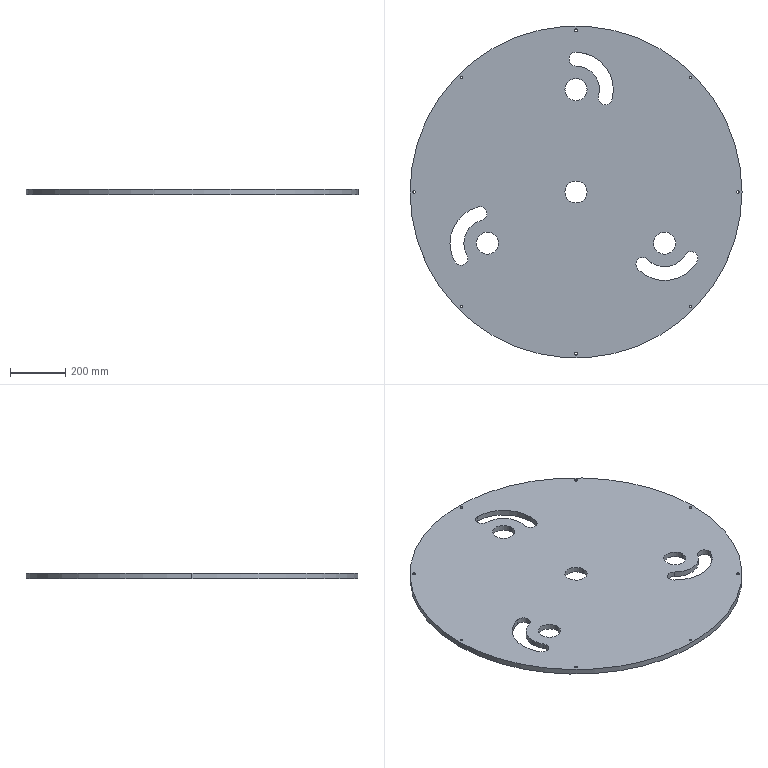Part | SolidWorks | features Extrusion 1 | 1 solid | 45 faces | box 1200 x 1200 x 20 mm | volume 21477450 mm3 | cylinder 43 | plane 2 | commonest cylinder face diameters 10 x16 50 x9 80 x8 170 x4 270 x4 1200 x2
STEP:
#1=CARTESIAN_POINT('',(-418.657,413.657,20.));
#2=VERTEX_POINT('',#1);
#3=CARTESIAN_POINT('',(-408.657,413.657,20.));
#4=VERTEX_POINT('',#3);
#5=CARTESIAN_POINT('',(-413.657,413.657,20.));
#6=DIRECTION('',(0.,0.,1.));
#7=DIRECTION('',(1.,0.,0.));
#8=AXIS2_PLACEMENT_3D('',#5,#6,#7);
#9=CIRCLE('',#8,5.);
#10=EDGE_CURVE('',#2,#4,#9,.T.);
#11=ORIENTED_EDGE('',*,*,#10,.T.);
#12=CARTESIAN_POINT('',(-408.657,413.657,0.));
#13=VERTEX_POINT('',#12);
#14=CARTESIAN_POINT('',(-408.657,413.657,20.));
#15=DIRECTION('',(0.,0.,-1.));
#16=VECTOR('',#15,1000.);
#17=LINE('',#14,#16);
#18=EDGE_CURVE('',#4,#13,#17,.T.);
#19=ORIENTED_EDGE('',*,*,#18,.T.);
#20=CARTESIAN_POINT('',(-418.657,413.657,0.));
#21=VERTEX_POINT('',#20);
#22=CARTESIAN_POINT('',(-413.657,413.657,0.));
#23=DIRECTION('',(0.,0.,1.));
#24=DIRECTION('',(1.,0.,0.));
#25=AXIS2_PLACEMENT_3D('',#22,#23,#24);
#26=CIRCLE('',#25,5.);
#27=EDGE_CURVE('',#21,#13,#26,.T.);
#28=ORIENTED_EDGE('',*,*,#27,.F.);
#29=CARTESIAN_POINT('',(-418.657,413.657,20.));
#30=DIRECTION('',(0.,0.,-1.));
#31=VECTOR('',#30,1000.);
#32=LINE('',#29,#31);
#33=EDGE_CURVE('',#2,#21,#32,.T.);
#34=ORIENTED_EDGE('',*,*,#33,.F.);
#35=EDGE_LOOP('',(#11,#19,#28,#34));
#36=FACE_OUTER_BOUND('',#35,.T.);
#37=CARTESIAN_POINT('',(-413.657,413.657,20.));
#38=DIRECTION('',(0.,0.,-1.));
#39=DIRECTION('',(-1.,0.,0.));
#40=AXIS2_PLACEMENT_3D('',#37,#38,#39);
#41=CYLINDRICAL_SURFACE('',#40,5.);
#42=ADVANCED_FACE('',(#36),#41,.F.);
#43=CARTESIAN_POINT('',(-590.,0.,20.));
#44=VERTEX_POINT('',#43);
#45=CARTESIAN_POINT('',(-580.,0.,20.));
#46=VERTEX_POINT('',#45);
#47=CARTESIAN_POINT('',(-585.,0.,20.));
#48=DIRECTION('',(0.,0.,1.));
#49=DIRECTION('',(1.,0.,0.));
#50=AXIS2_PLACEMENT_3D('',#47,#48,#49);
#51=CIRCLE('',#50,5.);
#52=EDGE_CURVE('',#44,#46,#51,.T.);
#53=ORIENTED_EDGE('',*,*,#52,.T.);
#54=CARTESIAN_POINT('',(-580.,0.,0.));
#55=VERTEX_POINT('',#54);
#56=CARTESIAN_POINT('',(-580.,0.,20.));
#57=DIRECTION('',(0.,0.,-1.));
#58=VECTOR('',#57,1000.);
#59=LINE('',#56,#58);
#60=EDGE_CURVE('',#46,#55,#59,.T.);
#61=ORIENTED_EDGE('',*,*,#60,.T.);
#62=CARTESIAN_POINT('',(-590.,0.,0.));
#63=VERTEX_POINT('',#62);
#64=CARTESIAN_POINT('',(-585.,0.,0.));
#65=DIRECTION('',(0.,0.,1.));
#66=DIRECTION('',(1.,0.,0.));
#67=AXIS2_PLACEMENT_3D('',#64,#65,#66);
#68=CIRCLE('',#67,5.);
#69=EDGE_CURVE('',#63,#55,#68,.T.);
#70=ORIENTED_EDGE('',*,*,#69,.F.);
#71=CARTESIAN_POINT('',(-590.,0.,20.));
#72=DIRECTION('',(0.,0.,-1.));
#73=VECTOR('',#72,1000.);
#74=LINE('',#71,#73);
#75=EDGE_CURVE('',#44,#63,#74,.T.);
#76=ORIENTED_EDGE('',*,*,#75,.F.);
#77=EDGE_LOOP('',(#53,#61,#70,#76));
#78=FACE_OUTER_BOUND('',#77,.T.);
#79=CARTESIAN_POINT('',(-585.,0.,20.));
#80=DIRECTION('',(0.,0.,-1.));
#81=DIRECTION('',(-1.,0.,0.));
#82=AXIS2_PLACEMENT_3D('',#79,#80,#81);
#83=CYLINDRICAL_SURFACE('',#82,5.);
#84=ADVANCED_FACE('',(#78),#83,.F.);
#85=CARTESIAN_POINT('',(-418.657,-413.657,20.));
#86=VERTEX_POINT('',#85);
#87=CARTESIAN_POINT('',(-408.657,-413.657,20.));
#88=VERTEX_POINT('',#87);
#89=CARTESIAN_POINT('',(-413.657,-413.657,20.));
#90=DIRECTION('',(0.,0.,1.));
#91=DIRECTION('',(1.,0.,0.));
#92=AXIS2_PLACEMENT_3D('',#89,#90,#91);
#93=CIRCLE('',#92,5.);
#94=EDGE_CURVE('',#86,#88,#93,.T.);
#95=ORIENTED_EDGE('',*,*,#94,.T.);
#96=CARTESIAN_POINT('',(-408.657,-413.657,0.));
#97=VERTEX_POINT('',#96);
#98=CARTESIAN_POINT('',(-408.657,-413.657,20.));
#99=DIRECTION('',(0.,0.,-1.));
#100=VECTOR('',#99,1000.);
#101=LINE('',#98,#100);
#102=EDGE_CURVE('',#88,#97,#101,.T.);
#103=ORIENTED_EDGE('',*,*,#102,.T.);
#104=CARTESIAN_POINT('',(-418.657,-413.657,0.));
#105=VERTEX_POINT('',#104);
#106=CARTESIAN_POINT('',(-413.657,-413.657,0.));
#107=DIRECTION('',(0.,0.,1.));
#108=DIRECTION('',(1.,0.,0.));
#109=AXIS2_PLACEMENT_3D('',#106,#107,#108);
#110=CIRCLE('',#109,5.);
#111=EDGE_CURVE('',#105,#97,#110,.T.);
#112=ORIENTED_EDGE('',*,*,#111,.F.);
#113=CARTESIAN_POINT('',(-418.657,-413.657,20.));
#114=DIRECTION('',(0.,0.,-1.));
#115=VECTOR('',#114,1000.);
#116=LINE('',#113,#115);
#117=EDGE_CURVE('',#86,#105,#116,.T.);
#118=ORIENTED_EDGE('',*,*,#117,.F.);
#119=EDGE_LOOP('',(#95,#103,#112,#118));
#120=FACE_OUTER_BOUND('',#119,.T.);
#121=CARTESIAN_POINT('',(-413.657,-413.657,20.));
#122=DIRECTION('',(0.,0.,-1.));
#123=DIRECTION('',(-1.,0.,0.));
#124=AXIS2_PLACEMENT_3D('',#121,#122,#123);
#125=CYLINDRICAL_SURFACE('',#124,5.);
#126=ADVANCED_FACE('',(#120),#125,.F.);
#127=CARTESIAN_POINT('',(-5.,-585.,20.));
#128=VERTEX_POINT('',#127);
#129=CARTESIAN_POINT('',(5.,-585.,20.));
#130=VERTEX_POINT('',#129);
#131=CARTESIAN_POINT('',(0.,-585.,20.));
#132=DIRECTION('',(0.,0.,1.));
#133=DIRECTION('',(1.,0.,0.));
#134=AXIS2_PLACEMENT_3D('',#131,#132,#133);
#135=CIRCLE('',#134,5.);
#136=EDGE_CURVE('',#128,#130,#135,.T.);
#137=ORIENTED_EDGE('',*,*,#136,.T.);
#138=CARTESIAN_POINT('',(5.,-585.,0.));
#139=VERTEX_POINT('',#138);
#140=CARTESIAN_POINT('',(5.,-585.,20.));
#141=DIRECTION('',(0.,0.,-1.));
#142=VECTOR('',#141,1000.);
#143=LINE('',#140,#142);
#144=EDGE_CURVE('',#130,#139,#143,.T.);
#145=ORIENTED_EDGE('',*,*,#144,.T.);
#146=CARTESIAN_POINT('',(-5.,-585.,0.));
#147=VERTEX_POINT('',#146);
#148=CARTESIAN_POINT('',(0.,-585.,0.));
#149=DIRECTION('',(0.,0.,1.));
#150=DIRECTION('',(1.,0.,0.));
#151=AXIS2_PLACEMENT_3D('',#148,#149,#150);
#152=CIRCLE('',#151,5.);
#153=EDGE_CURVE('',#147,#139,#152,.T.);
#154=ORIENTED_EDGE('',*,*,#153,.F.);
#155=CARTESIAN_POINT('',(-5.,-585.,20.));
#156=DIRECTION('',(0.,0.,-1.));
#157=VECTOR('',#156,1000.);
#158=LINE('',#155,#157);
#159=EDGE_CURVE('',#128,#147,#158,.T.);
#160=ORIENTED_EDGE('',*,*,#159,.F.);
#161=EDGE_LOOP('',(#137,#145,#154,#160));
#162=FACE_OUTER_BOUND('',#161,.T.);
#163=CARTESIAN_POINT('',(0.,-585.,20.));
#164=DIRECTION('',(0.,0.,-1.));
#165=DIRECTION('',(-1.,0.,0.));
#166=AXIS2_PLACEMENT_3D('',#163,#164,#165);
#167=CYLINDRICAL_SURFACE('',#166,5.);
#168=ADVANCED_FACE('',(#162),#167,.F.);
#169=CARTESIAN_POINT('',(408.657,-413.657,20.));
#170=VERTEX_POINT('',#169);
#171=CARTESIAN_POINT('',(418.657,-413.657,20.));
#172=VERTEX_POINT('',#171);
#173=CARTESIAN_POINT('',(413.657,-413.657,20.));
#174=DIRECTION('',(0.,0.,1.));
#175=DIRECTION('',(1.,0.,0.));
#176=AXIS2_PLACEMENT_3D('',#173,#174,#175);
#177=CIRCLE('',#176,5.);
#178=EDGE_CURVE('',#170,#172,#177,.T.);
#179=ORIENTED_EDGE('',*,*,#178,.T.);
#180=CARTESIAN_POINT('',(418.657,-413.657,0.));
#181=VERTEX_POINT('',#180);
#182=CARTESIAN_POINT('',(418.657,-413.657,20.));
#183=DIRECTION('',(0.,0.,-1.));
#184=VECTOR('',#183,1000.);
#185=LINE('',#182,#184);
#186=EDGE_CURVE('',#172,#181,#185,.T.);
#187=ORIENTED_EDGE('',*,*,#186,.T.);
#188=CARTESIAN_POINT('',(408.657,-413.657,0.));
#189=VERTEX_POINT('',#188);
#190=CARTESIAN_POINT('',(413.657,-413.657,0.));
#191=DIRECTION('',(0.,0.,1.));
#192=DIRECTION('',(1.,0.,0.));
#193=AXIS2_PLACEMENT_3D('',#190,#191,#192);
#194=CIRCLE('',#193,5.);
#195=EDGE_CURVE('',#189,#181,#194,.T.);
#196=ORIENTED_EDGE('',*,*,#195,.F.);
#197=CARTESIAN_POINT('',(408.657,-413.657,20.));
#198=DIRECTION('',(0.,0.,-1.));
#199=VECTOR('',#198,1000.);
#200=LINE('',#197,#199);
#201=EDGE_CURVE('',#170,#189,#200,.T.);
#202=ORIENTED_EDGE('',*,*,#201,.F.);
#203=EDGE_LOOP('',(#179,#187,#196,#202));
#204=FACE_OUTER_BOUND('',#203,.T.);
#205=CARTESIAN_POINT('',(413.657,-413.657,20.));
#206=DIRECTION('',(0.,0.,-1.));
#207=DIRECTION('',(-1.,0.,0.));
#208=AXIS2_PLACEMENT_3D('',#205,#206,#207);
#209=CYLINDRICAL_SURFACE('',#208,5.);
#210=ADVANCED_FACE('',(#204),#209,.F.);
#211=CARTESIAN_POINT('',(580.,0.,20.));
#212=VERTEX_POINT('',#211);
#213=CARTESIAN_POINT('',(590.,0.,20.));
#214=VERTEX_POINT('',#213);
#215=CARTESIAN_POINT('',(585.,0.,20.));
#216=DIRECTION('',(0.,0.,1.));
#217=DIRECTION('',(1.,0.,0.));
#218=AXIS2_PLACEMENT_3D('',#215,#216,#217);
#219=CIRCLE('',#218,5.);
#220=EDGE_CURVE('',#212,#214,#219,.T.);
#221=ORIENTED_EDGE('',*,*,#220,.T.);
#222=CARTESIAN_POINT('',(590.,0.,0.));
#223=VERTEX_POINT('',#222);
#224=CARTESIAN_POINT('',(590.,0.,20.));
#225=DIRECTION('',(0.,0.,-1.));
#226=VECTOR('',#225,1000.);
#227=LINE('',#224,#226);
#228=EDGE_CURVE('',#214,#223,#227,.T.);
#229=ORIENTED_EDGE('',*,*,#228,.T.);
#230=CARTESIAN_POINT('',(580.,0.,0.));
#231=VERTEX_POINT('',#230);
#232=CARTESIAN_POINT('',(585.,0.,0.));
#233=DIRECTION('',(0.,0.,1.));
#234=DIRECTION('',(1.,0.,0.));
#235=AXIS2_PLACEMENT_3D('',#232,#233,#234);
#236=CIRCLE('',#235,5.);
#237=EDGE_CURVE('',#231,#223,#236,.T.);
#238=ORIENTED_EDGE('',*,*,#237,.F.);
#239=CARTESIAN_POINT('',(580.,0.,20.));
#240=DIRECTION('',(0.,0.,-1.));
#241=VECTOR('',#240,1000.);
#242=LINE('',#239,#241);
#243=EDGE_CURVE('',#212,#231,#242,.T.);
#244=ORIENTED_EDGE('',*,*,#243,.F.);
#245=EDGE_LOOP('',(#221,#229,#238,#244));
#246=FACE_OUTER_BOUND('',#245,.T.);
#247=CARTESIAN_POINT('',(585.,0.,20.));
#248=DIRECTION('',(0.,0.,-1.));
#249=DIRECTION('',(-1.,0.,0.));
#250=AXIS2_PLACEMENT_3D('',#247,#248,#249);
#251=CYLINDRICAL_SURFACE('',#250,5.);
#252=ADVANCED_FACE('',(#246),#251,.F.);
#253=CARTESIAN_POINT('',(408.657,413.657,20.));
#254=VERTEX_POINT('',#253);
#255=CARTESIAN_POINT('',(418.657,413.657,20.));
#256=VERTEX_POINT('',#255);
#257=CARTESIAN_POINT('',(413.657,413.657,20.));
#258=DIRECTION('',(0.,0.,1.));
#259=DIRECTION('',(1.,0.,0.));
#260=AXIS2_PLACEMENT_3D('',#257,#258,#259);
#261=CIRCLE('',#260,5.);
#262=EDGE_CURVE('',#254,#256,#261,.T.);
#263=ORIENTED_EDGE('',*,*,#262,.T.);
#264=CARTESIAN_POINT('',(418.657,413.657,0.));
#265=VERTEX_POINT('',#264);
#266=CARTESIAN_POINT('',(418.657,413.657,20.));
#267=DIRECTION('',(0.,0.,-1.));
#268=VECTOR('',#267,1000.);
#269=LINE('',#266,#268);
#270=EDGE_CURVE('',#256,#265,#269,.T.);
#271=ORIENTED_EDGE('',*,*,#270,.T.);
#272=CARTESIAN_POINT('',(408.657,413.657,0.));
#273=VERTEX_POINT('',#272);
#274=CARTESIAN_POINT('',(413.657,413.657,0.));
#275=DIRECTION('',(0.,0.,1.));
#276=DIRECTION('',(1.,0.,0.));
#277=AXIS2_PLACEMENT_3D('',#274,#275,#276);
#278=CIRCLE('',#277,5.);
#279=EDGE_CURVE('',#273,#265,#278,.T.);
#280=ORIENTED_EDGE('',*,*,#279,.F.);
#281=CARTESIAN_POINT('',(408.657,413.657,20.));
#282=DIRECTION('',(0.,0.,-1.));
#283=VECTOR('',#282,1000.);
#284=LINE('',#281,#283);
#285=EDGE_CURVE('',#254,#273,#284,.T.);
#286=ORIENTED_EDGE('',*,*,#285,.F.);
#287=EDGE_LOOP('',(#263,#271,#280,#286));
#288=FACE_OUTER_BOUND('',#287,.T.);
#289=CARTESIAN_POINT('',(413.657,413.657,20.));
#290=DIRECTION('',(0.,0.,-1.));
#291=DIRECTION('',(-1.,0.,0.));
#292=AXIS2_PLACEMENT_3D('',#289,#290,#291);
#293=CYLINDRICAL_SURFACE('',#292,5.);
#294=ADVANCED_FACE('',(#288),#293,.F.);
#295=CARTESIAN_POINT('',(-394.042,-227.5,20.));
#296=VERTEX_POINT('',#295);
#297=CARTESIAN_POINT('',(-405.429,-185.,20.));
#298=VERTEX_POINT('',#297);
#299=CARTESIAN_POINT('',(-320.429,-185.,20.));
#300=DIRECTION('',(0.,0.,-1.));
#301=DIRECTION('',(1.,0.,0.));
#302=AXIS2_PLACEMENT_3D('',#299,#300,#301);
#303=CIRCLE('',#302,85.);
#304=EDGE_CURVE('',#296,#298,#303,.T.);
#305=ORIENTED_EDGE('',*,*,#304,.T.);
#306=CARTESIAN_POINT('',(-405.429,-185.,0.));
#307=VERTEX_POINT('',#306);
#308=CARTESIAN_POINT('',(-405.429,-185.,20.));
#309=DIRECTION('',(0.,0.,-1.));
#310=VECTOR('',#309,1000.);
#311=LINE('',#308,#310);
#312=EDGE_CURVE('',#298,#307,#311,.T.);
#313=ORIENTED_EDGE('',*,*,#312,.T.);
#314=CARTESIAN_POINT('',(-394.042,-227.5,0.));
#315=VERTEX_POINT('',#314);
#316=CARTESIAN_POINT('',(-320.429,-185.,0.));
#317=DIRECTION('',(0.,0.,-1.));
#318=DIRECTION('',(1.,0.,0.));
#319=AXIS2_PLACEMENT_3D('',#316,#317,#318);
#320=CIRCLE('',#319,85.);
#321=EDGE_CURVE('',#315,#307,#320,.T.);
#322=ORIENTED_EDGE('',*,*,#321,.F.);
#323=CARTESIAN_POINT('',(-394.042,-227.5,20.));
#324=DIRECTION('',(0.,0.,-1.));
#325=VECTOR('',#324,1000.);
#326=LINE('',#323,#325);
#327=EDGE_CURVE('',#296,#315,#326,.T.);
#328=ORIENTED_EDGE('',*,*,#327,.F.);
#329=EDGE_LOOP('',(#305,#313,#322,#328));
#330=FACE_OUTER_BOUND('',#329,.T.);
#331=CARTESIAN_POINT('',(-320.429,-185.,20.));
#332=DIRECTION('',(0.,0.,-1.));
#333=DIRECTION('',(-1.,0.,0.));
#334=AXIS2_PLACEMENT_3D('',#331,#332,#333);
#335=CYLINDRICAL_SURFACE('',#334,85.);
#336=ADVANCED_FACE('',(#330),#335,.T.);
#337=CARTESIAN_POINT('',(-353.485,-54.11,20.));
#338=VERTEX_POINT('',#337);
#339=CARTESIAN_POINT('',(-455.429,-185.,20.));
#340=VERTEX_POINT('',#339);
#341=CARTESIAN_POINT('',(-320.429,-185.,20.));
#342=DIRECTION('',(0.,0.,1.));
#343=DIRECTION('',(1.,0.,0.));
#344=AXIS2_PLACEMENT_3D('',#341,#342,#343);
#345=CIRCLE('',#344,135.);
#346=EDGE_CURVE('',#338,#340,#345,.T.);
#347=ORIENTED_EDGE('',*,*,#346,.T.);
#348=CARTESIAN_POINT('',(-455.429,-185.,0.));
#349=VERTEX_POINT('',#348);
#350=CARTESIAN_POINT('',(-455.429,-185.,20.));
#351=DIRECTION('',(0.,0.,-1.));
#352=VECTOR('',#351,1000.);
#353=LINE('',#350,#352);
#354=EDGE_CURVE('',#340,#349,#353,.T.);
#355=ORIENTED_EDGE('',*,*,#354,.T.);
#356=CARTESIAN_POINT('',(-353.485,-54.11,0.));
#357=VERTEX_POINT('',#356);
#358=CARTESIAN_POINT('',(-320.429,-185.,0.));
#359=DIRECTION('',(0.,0.,1.));
#360=DIRECTION('',(1.,0.,0.));
#361=AXIS2_PLACEMENT_3D('',#358,#359,#360);
#362=CIRCLE('',#361,135.);
#363=EDGE_CURVE('',#357,#349,#362,.T.);
#364=ORIENTED_EDGE('',*,*,#363,.F.);
#365=CARTESIAN_POINT('',(-353.485,-54.11,20.));
#366=DIRECTION('',(0.,0.,-1.));
#367=VECTOR('',#366,1000.);
#368=LINE('',#365,#367);
#369=EDGE_CURVE('',#338,#357,#368,.T.);
#370=ORIENTED_EDGE('',*,*,#369,.F.);
#371=EDGE_LOOP('',(#347,#355,#364,#370));
#372=FACE_OUTER_BOUND('',#371,.T.);
#373=CARTESIAN_POINT('',(-320.429,-185.,20.));
#374=DIRECTION('',(0.,0.,-1.));
#375=DIRECTION('',(-1.,0.,0.));
#376=AXIS2_PLACEMENT_3D('',#373,#374,#375);
#377=CYLINDRICAL_SURFACE('',#376,135.);
#378=ADVANCED_FACE('',(#372),#377,.F.);
#379=CARTESIAN_POINT('',(259.464,-244.231,20.));
#380=VERTEX_POINT('',#379);
#381=CARTESIAN_POINT('',(216.534,-261.652,20.));
#382=VERTEX_POINT('',#381);
#383=CARTESIAN_POINT('',(241.534,-261.652,20.));
#384=DIRECTION('',(0.,0.,1.));
#385=DIRECTION('',(1.,0.,0.));
#386=AXIS2_PLACEMENT_3D('',#383,#384,#385);
#387=CIRCLE('',#386,25.);
#388=EDGE_CURVE('',#380,#382,#387,.T.);
#389=ORIENTED_EDGE('',*,*,#388,.T.);
#390=CARTESIAN_POINT('',(216.534,-261.652,0.));
#391=VERTEX_POINT('',#390);
#392=CARTESIAN_POINT('',(216.534,-261.652,20.));
#393=DIRECTION('',(0.,0.,-1.));
#394=VECTOR('',#393,1000.);
#395=LINE('',#392,#394);
#396=EDGE_CURVE('',#382,#391,#395,.T.);
#397=ORIENTED_EDGE('',*,*,#396,.T.);
#398=CARTESIAN_POINT('',(259.464,-244.231,0.));
#399=VERTEX_POINT('',#398);
#400=CARTESIAN_POINT('',(241.534,-261.652,0.));
#401=DIRECTION('',(0.,0.,1.));
#402=DIRECTION('',(1.,0.,0.));
#403=AXIS2_PLACEMENT_3D('',#400,#401,#402);
#404=CIRCLE('',#403,25.);
#405=EDGE_CURVE('',#399,#391,#404,.T.);
#406=ORIENTED_EDGE('',*,*,#405,.F.);
#407=CARTESIAN_POINT('',(259.464,-244.231,20.));
#408=DIRECTION('',(0.,0.,-1.));
#409=VECTOR('',#408,1000.);
#410=LINE('',#407,#409);
#411=EDGE_CURVE('',#380,#399,#410,.T.);
#412=ORIENTED_EDGE('',*,*,#411,.F.);
#413=EDGE_LOOP('',(#389,#397,#406,#412));
#414=FACE_OUTER_BOUND('',#413,.T.);
#415=CARTESIAN_POINT('',(241.534,-261.652,20.));
#416=DIRECTION('',(0.,0.,-1.));
#417=DIRECTION('',(-1.,0.,0.));
#418=AXIS2_PLACEMENT_3D('',#415,#416,#417);
#419=CYLINDRICAL_SURFACE('',#418,25.);
#420=ADVANCED_FACE('',(#414),#419,.F.);
#421=CARTESIAN_POINT('',(-5.,585.,20.));
#422=VERTEX_POINT('',#421);
#423=CARTESIAN_POINT('',(5.,585.,20.));
#424=VERTEX_POINT('',#423);
#425=CARTESIAN_POINT('',(0.,585.,20.));
#426=DIRECTION('',(0.,0.,1.));
#427=DIRECTION('',(1.,0.,0.));
#428=AXIS2_PLACEMENT_3D('',#425,#426,#427);
#429=CIRCLE('',#428,5.);
#430=EDGE_CURVE('',#422,#424,#429,.T.);
#431=ORIENTED_EDGE('',*,*,#430,.T.);
#432=CARTESIAN_POINT('',(5.,585.,0.));
#433=VERTEX_POINT('',#432);
#434=CARTESIAN_POINT('',(5.,585.,20.));
#435=DIRECTION('',(0.,0.,-1.));
#436=VECTOR('',#435,1000.);
#437=LINE('',#434,#436);
#438=EDGE_CURVE('',#424,#433,#437,.T.);
#439=ORIENTED_EDGE('',*,*,#438,.T.);
#440=CARTESIAN_POINT('',(-5.,585.,0.));
#441=VERTEX_POINT('',#440);
#442=CARTESIAN_POINT('',(0.,585.,0.));
#443=DIRECTION('',(0.,0.,1.));
#444=DIRECTION('',(1.,0.,0.));
#445=AXIS2_PLACEMENT_3D('',#442,#443,#444);
#446=CIRCLE('',#445,5.);
#447=EDGE_CURVE('',#441,#433,#446,.T.);
#448=ORIENTED_EDGE('',*,*,#447,.F.);
#449=CARTESIAN_POINT('',(-5.,585.,20.));
#450=DIRECTION('',(0.,0.,-1.));
#451=VECTOR('',#450,1000.);
#452=LINE('',#449,#451);
#453=EDGE_CURVE('',#422,#441,#452,.T.);
#454=ORIENTED_EDGE('',*,*,#453,.F.);
#455=EDGE_LOOP('',(#431,#439,#448,#454));
#456=FACE_OUTER_BOUND('',#455,.T.);
#457=CARTESIAN_POINT('',(0.,585.,20.));
#458=DIRECTION('',(0.,0.,-1.));
#459=DIRECTION('',(-1.,0.,0.));
#460=AXIS2_PLACEMENT_3D('',#457,#458,#459);
#461=CYLINDRICAL_SURFACE('',#460,5.);
#462=ADVANCED_FACE('',(#456),#461,.F.);
#463=CARTESIAN_POINT('',(0.,505.,20.));
#464=VERTEX_POINT('',#463);
#465=CARTESIAN_POINT('',(-25.,480.,20.));
#466=VERTEX_POINT('',#465);
#467=CARTESIAN_POINT('',(0.,480.,20.));
#468=DIRECTION('',(0.,0.,1.));
#469=DIRECTION('',(1.,0.,0.));
#470=AXIS2_PLACEMENT_3D('',#467,#468,#469);
#471=CIRCLE('',#470,25.);
#472=EDGE_CURVE('',#464,#466,#471,.T.);
#473=ORIENTED_EDGE('',*,*,#472,.T.);
#474=CARTESIAN_POINT('',(-25.,480.,0.));
#475=VERTEX_POINT('',#474);
#476=CARTESIAN_POINT('',(-25.,480.,20.));
#477=DIRECTION('',(0.,0.,-1.));
#478=VECTOR('',#477,1000.);
#479=LINE('',#476,#478);
#480=EDGE_CURVE('',#466,#475,#479,.T.);
#481=ORIENTED_EDGE('',*,*,#480,.T.);
#482=CARTESIAN_POINT('',(0.,505.,0.));
#483=VERTEX_POINT('',#482);
#484=CARTESIAN_POINT('',(0.,480.,0.));
#485=DIRECTION('',(0.,0.,1.));
#486=DIRECTION('',(1.,0.,0.));
#487=AXIS2_PLACEMENT_3D('',#484,#485,#486);
#488=CIRCLE('',#487,25.);
#489=EDGE_CURVE('',#483,#475,#488,.T.);
#490=ORIENTED_EDGE('',*,*,#489,.F.);
#491=CARTESIAN_POINT('',(0.,505.,20.));
#492=DIRECTION('',(0.,0.,-1.));
#493=VECTOR('',#492,1000.);
#494=LINE('',#491,#493);
#495=EDGE_CURVE('',#464,#483,#494,.T.);
#496=ORIENTED_EDGE('',*,*,#495,.F.);
#497=EDGE_LOOP('',(#473,#481,#490,#496));
#498=FACE_OUTER_BOUND('',#497,.T.);
#499=CARTESIAN_POINT('',(0.,480.,20.));
#500=DIRECTION('',(0.,0.,-1.));
#501=DIRECTION('',(-1.,0.,0.));
#502=AXIS2_PLACEMENT_3D('',#499,#500,#501);
#503=CYLINDRICAL_SURFACE('',#502,25.);
#504=ADVANCED_FACE('',(#498),#503,.F.);
#505=CARTESIAN_POINT('',(81.778,346.818,20.));
#506=VERTEX_POINT('',#505);
#507=CARTESIAN_POINT('',(80.83,340.,20.));
#508=VERTEX_POINT('',#507);
#509=CARTESIAN_POINT('',(105.83,340.,20.));
#510=DIRECTION('',(0.,0.,1.));
#511=DIRECTION('',(1.,0.,0.));
#512=AXIS2_PLACEMENT_3D('',#509,#510,#511);
#513=CIRCLE('',#512,25.);
#514=EDGE_CURVE('',#506,#508,#513,.T.);
#515=ORIENTED_EDGE('',*,*,#514,.T.);
#516=CARTESIAN_POINT('',(80.83,340.,0.));
#517=VERTEX_POINT('',#516);
#518=CARTESIAN_POINT('',(80.83,340.,20.));
#519=DIRECTION('',(0.,0.,-1.));
#520=VECTOR('',#519,1000.);
#521=LINE('',#518,#520);
#522=EDGE_CURVE('',#508,#517,#521,.T.);
#523=ORIENTED_EDGE('',*,*,#522,.T.);
#524=CARTESIAN_POINT('',(81.778,346.818,0.));
#525=VERTEX_POINT('',#524);
#526=CARTESIAN_POINT('',(105.83,340.,0.));
#527=DIRECTION('',(0.,0.,1.));
#528=DIRECTION('',(1.,0.,0.));
#529=AXIS2_PLACEMENT_3D('',#526,#527,#528);
#530=CIRCLE('',#529,25.);
#531=EDGE_CURVE('',#525,#517,#530,.T.);
#532=ORIENTED_EDGE('',*,*,#531,.F.);
#533=CARTESIAN_POINT('',(81.778,346.818,20.));
#534=DIRECTION('',(0.,0.,-1.));
#535=VECTOR('',#534,1000.);
#536=LINE('',#533,#535);
#537=EDGE_CURVE('',#506,#525,#536,.T.);
#538=ORIENTED_EDGE('',*,*,#537,.F.);
#539=EDGE_LOOP('',(#515,#523,#532,#538));
#540=FACE_OUTER_BOUND('',#539,.T.);
#541=CARTESIAN_POINT('',(105.83,340.,20.));
#542=DIRECTION('',(0.,0.,-1.));
#543=DIRECTION('',(-1.,0.,0.));
#544=AXIS2_PLACEMENT_3D('',#541,#542,#543);
#545=CYLINDRICAL_SURFACE('',#544,25.);
#546=ADVANCED_FACE('',(#540),#545,.F.);
#547=CARTESIAN_POINT('',(-360.429,-185.,20.));
#548=VERTEX_POINT('',#547);
#549=CARTESIAN_POINT('',(-280.429,-185.,20.));
#550=VERTEX_POINT('',#549);
#551=CARTESIAN_POINT('',(-320.429,-185.,20.));
#552=DIRECTION('',(0.,0.,1.));
#553=DIRECTION('',(1.,0.,0.));
#554=AXIS2_PLACEMENT_3D('',#551,#552,#553);
#555=CIRCLE('',#554,40.);
#556=EDGE_CURVE('',#548,#550,#555,.T.);
#557=ORIENTED_EDGE('',*,*,#556,.T.);
#558=CARTESIAN_POINT('',(-280.429,-185.,0.));
#559=VERTEX_POINT('',#558);
#560=CARTESIAN_POINT('',(-280.429,-185.,20.));
#561=DIRECTION('',(0.,0.,-1.));
#562=VECTOR('',#561,1000.);
#563=LINE('',#560,#562);
#564=EDGE_CURVE('',#550,#559,#563,.T.);
#565=ORIENTED_EDGE('',*,*,#564,.T.);
#566=CARTESIAN_POINT('',(-360.429,-185.,0.));
#567=VERTEX_POINT('',#566);
#568=CARTESIAN_POINT('',(-320.429,-185.,0.));
#569=DIRECTION('',(0.,0.,1.));
#570=DIRECTION('',(1.,0.,0.));
#571=AXIS2_PLACEMENT_3D('',#568,#569,#570);
#572=CIRCLE('',#571,40.);
#573=EDGE_CURVE('',#567,#559,#572,.T.);
#574=ORIENTED_EDGE('',*,*,#573,.F.);
#575=CARTESIAN_POINT('',(-360.429,-185.,20.));
#576=DIRECTION('',(0.,0.,-1.));
#577=VECTOR('',#576,1000.);
#578=LINE('',#575,#577);
#579=EDGE_CURVE('',#548,#567,#578,.T.);
#580=ORIENTED_EDGE('',*,*,#579,.F.);
#581=EDGE_LOOP('',(#557,#565,#574,#580));
#582=FACE_OUTER_BOUND('',#581,.T.);
#583=CARTESIAN_POINT('',(-320.429,-185.,20.));
#584=DIRECTION('',(0.,0.,-1.));
#585=DIRECTION('',(-1.,0.,0.));
#586=AXIS2_PLACEMENT_3D('',#583,#584,#585);
#587=CYLINDRICAL_SURFACE('',#586,40.);
#588=ADVANCED_FACE('',(#582),#587,.F.);
#589=CARTESIAN_POINT('',(280.429,-185.,20.));
#590=VERTEX_POINT('',#589);
#591=CARTESIAN_POINT('',(360.429,-185.,20.));
#592=VERTEX_POINT('',#591);
#593=CARTESIAN_POINT('',(320.429,-185.,20.));
#594=DIRECTION('',(0.,0.,1.));
#595=DIRECTION('',(1.,0.,0.));
#596=AXIS2_PLACEMENT_3D('',#593,#594,#595);
#597=CIRCLE('',#596,40.);
#598=EDGE_CURVE('',#590,#592,#597,.T.);
#599=ORIENTED_EDGE('',*,*,#598,.T.);
#600=CARTESIAN_POINT('',(360.429,-185.,0.));
#601=VERTEX_POINT('',#600);
#602=CARTESIAN_POINT('',(360.429,-185.,20.));
#603=DIRECTION('',(0.,0.,-1.));
#604=VECTOR('',#603,1000.);
#605=LINE('',#602,#604);
#606=EDGE_CURVE('',#592,#601,#605,.T.);
#607=ORIENTED_EDGE('',*,*,#606,.T.);
#608=CARTESIAN_POINT('',(280.429,-185.,0.));
#609=VERTEX_POINT('',#608);
#610=CARTESIAN_POINT('',(320.429,-185.,0.));
#611=DIRECTION('',(0.,0.,1.));
#612=DIRECTION('',(1.,0.,0.));
#613=AXIS2_PLACEMENT_3D('',#610,#611,#612);
#614=CIRCLE('',#613,40.);
#615=EDGE_CURVE('',#609,#601,#614,.T.);
#616=ORIENTED_EDGE('',*,*,#615,.F.);
#617=CARTESIAN_POINT('',(280.429,-185.,20.));
#618=DIRECTION('',(0.,0.,-1.));
#619=VECTOR('',#618,1000.);
#620=LINE('',#617,#619);
#621=EDGE_CURVE('',#590,#609,#620,.T.);
#622=ORIENTED_EDGE('',*,*,#621,.F.);
#623=EDGE_LOOP('',(#599,#607,#616,#622));
#624=FACE_OUTER_BOUND('',#623,.T.);
#625=CARTESIAN_POINT('',(320.429,-185.,20.));
#626=DIRECTION('',(0.,0.,-1.));
#627=DIRECTION('',(-1.,0.,0.));
#628=AXIS2_PLACEMENT_3D('',#625,#626,#627);
#629=CYLINDRICAL_SURFACE('',#628,40.);
#630=ADVANCED_FACE('',(#624),#629,.F.);
#631=CARTESIAN_POINT('',(-40.,370.,20.));
#632=VERTEX_POINT('',#631);
#633=CARTESIAN_POINT('',(40.,370.,20.));
#634=VERTEX_POINT('',#633);
#635=CARTESIAN_POINT('',(0.,370.,20.));
#636=DIRECTION('',(0.,0.,1.));
#637=DIRECTION('',(1.,0.,0.));
#638=AXIS2_PLACEMENT_3D('',#635,#636,#637);
#639=CIRCLE('',#638,40.);
#640=EDGE_CURVE('',#632,#634,#639,.T.);
#641=ORIENTED_EDGE('',*,*,#640,.T.);
#642=CARTESIAN_POINT('',(40.,370.,0.));
#643=VERTEX_POINT('',#642);
#644=CARTESIAN_POINT('',(40.,370.,20.));
#645=DIRECTION('',(0.,0.,-1.));
#646=VECTOR('',#645,1000.);
#647=LINE('',#644,#646);
#648=EDGE_CURVE('',#634,#643,#647,.T.);
#649=ORIENTED_EDGE('',*,*,#648,.T.);
#650=CARTESIAN_POINT('',(-40.,370.,0.));
#651=VERTEX_POINT('',#650);
#652=CARTESIAN_POINT('',(0.,370.,0.));
#653=DIRECTION('',(0.,0.,1.));
#654=DIRECTION('',(1.,0.,0.));
#655=AXIS2_PLACEMENT_3D('',#652,#653,#654);
#656=CIRCLE('',#655,40.);
#657=EDGE_CURVE('',#651,#643,#656,.T.);
#658=ORIENTED_EDGE('',*,*,#657,.F.);
#659=CARTESIAN_POINT('',(-40.,370.,20.));
#660=DIRECTION('',(0.,0.,-1.));
#661=VECTOR('',#660,1000.);
#662=LINE('',#659,#661);
#663=EDGE_CURVE('',#632,#651,#662,.T.);
#664=ORIENTED_EDGE('',*,*,#663,.F.);
#665=EDGE_LOOP('',(#641,#649,#658,#664));
#666=FACE_OUTER_BOUND('',#665,.T.);
#667=CARTESIAN_POINT('',(0.,370.,20.));
#668=DIRECTION('',(0.,0.,-1.));
#669=DIRECTION('',(-1.,0.,0.));
#670=AXIS2_PLACEMENT_3D('',#667,#668,#669);
#671=CYLINDRICAL_SURFACE('',#670,40.);
#672=ADVANCED_FACE('',(#666),#671,.F.);
#673=CARTESIAN_POINT('',(-40.,0.,20.));
#674=VERTEX_POINT('',#673);
#675=CARTESIAN_POINT('',(40.,0.,20.));
#676=VERTEX_POINT('',#675);
#677=CARTESIAN_POINT('',(0.,0.,20.));
#678=DIRECTION('',(0.,0.,1.));
#679=DIRECTION('',(1.,0.,0.));
#680=AXIS2_PLACEMENT_3D('',#677,#678,#679);
#681=CIRCLE('',#680,40.);
#682=EDGE_CURVE('',#674,#676,#681,.T.);
#683=ORIENTED_EDGE('',*,*,#682,.T.);
#684=CARTESIAN_POINT('',(40.,0.,0.));
#685=VERTEX_POINT('',#684);
#686=CARTESIAN_POINT('',(40.,0.,20.));
#687=DIRECTION('',(0.,0.,-1.));
#688=VECTOR('',#687,1000.);
#689=LINE('',#686,#688);
#690=EDGE_CURVE('',#676,#685,#689,.T.);
#691=ORIENTED_EDGE('',*,*,#690,.T.);
#692=CARTESIAN_POINT('',(-40.,0.,0.));
#693=VERTEX_POINT('',#692);
#694=CARTESIAN_POINT('',(0.,0.,0.));
#695=DIRECTION('',(0.,0.,1.));
#696=DIRECTION('',(1.,0.,0.));
#697=AXIS2_PLACEMENT_3D('',#694,#695,#696);
#698=CIRCLE('',#697,40.);
#699=EDGE_CURVE('',#693,#685,#698,.T.);
#700=ORIENTED_EDGE('',*,*,#699,.F.);
#701=CARTESIAN_POINT('',(-40.,0.,20.));
#702=DIRECTION('',(0.,0.,-1.));
#703=VECTOR('',#702,1000.);
#704=LINE('',#701,#703);
#705=EDGE_CURVE('',#674,#693,#704,.T.);
#706=ORIENTED_EDGE('',*,*,#705,.F.);
#707=EDGE_LOOP('',(#683,#691,#700,#706));
#708=FACE_OUTER_BOUND('',#707,.T.);
#709=CARTESIAN_POINT('',(0.,0.,20.));
#710=DIRECTION('',(0.,0.,-1.));
#711=DIRECTION('',(-1.,0.,0.));
#712=AXIS2_PLACEMENT_3D('',#709,#710,#711);
#713=CYLINDRICAL_SURFACE('',#712,40.);
#714=ADVANCED_FACE('',(#708),#713,.F.);
#715=CARTESIAN_POINT('',(600.,0.,20.));
#716=VERTEX_POINT('',#715);
#717=CARTESIAN_POINT('',(-600.,0.,20.));
#718=VERTEX_POINT('',#717);
#719=CARTESIAN_POINT('',(0.,0.,20.));
#720=DIRECTION('',(0.,0.,1.));
#721=DIRECTION('',(1.,0.,0.));
#722=AXIS2_PLACEMENT_3D('',#719,#720,#721);
#723=CIRCLE('',#722,600.);
#724=EDGE_CURVE('',#716,#718,#723,.T.);
#725=ORIENTED_EDGE('',*,*,#724,.F.);
#726=CARTESIAN_POINT('',(600.,0.,0.));
#727=VERTEX_POINT('',#726);
#728=CARTESIAN_POINT('',(600.,0.,20.));
#729=DIRECTION('',(0.,0.,-1.));
#730=VECTOR('',#729,1000.);
#731=LINE('',#728,#730);
#732=EDGE_CURVE('',#716,#727,#731,.T.);
#733=ORIENTED_EDGE('',*,*,#732,.T.);
#734=CARTESIAN_POINT('',(-600.,0.,0.));
#735=VERTEX_POINT('',#734);
#736=CARTESIAN_POINT('',(0.,0.,0.));
#737=DIRECTION('',(0.,0.,1.));
#738=DIRECTION('',(1.,0.,0.));
#739=AXIS2_PLACEMENT_3D('',#736,#737,#738);
#740=CIRCLE('',#739,600.);
#741=EDGE_CURVE('',#727,#735,#740,.T.);
#742=ORIENTED_EDGE('',*,*,#741,.T.);
#743=CARTESIAN_POINT('',(-600.,0.,20.));
#744=DIRECTION('',(0.,0.,-1.));
#745=VECTOR('',#744,1000.);
#746=LINE('',#743,#745);
#747=EDGE_CURVE('',#718,#735,#746,.T.);
#748=ORIENTED_EDGE('',*,*,#747,.F.);
#749=EDGE_LOOP('',(#725,#733,#742,#748));
#750=FACE_OUTER_BOUND('',#749,.T.);
#751=CARTESIAN_POINT('',(0.,0.,20.));
#752=DIRECTION('',(0.,0.,-1.));
#753=DIRECTION('',(-1.,0.,0.));
#754=AXIS2_PLACEMENT_3D('',#751,#752,#753);
#755=CYLINDRICAL_SURFACE('',#754,600.);
#756=ADVANCED_FACE('',(#750),#755,.T.);
#757=ORIENTED_EDGE('',*,*,#52,.F.);
#758=CARTESIAN_POINT('',(-585.,0.,20.));
#759=DIRECTION('',(0.,0.,1.));
#760=DIRECTION('',(1.,0.,0.));
#761=AXIS2_PLACEMENT_3D('',#758,#759,#760);
#762=CIRCLE('',#761,5.);
#763=EDGE_CURVE('',#46,#44,#762,.T.);
#764=ORIENTED_EDGE('',*,*,#763,.F.);
#765=EDGE_LOOP('',(#757,#764));
#766=FACE_BOUND('',#765,.T.);
#767=ORIENTED_EDGE('',*,*,#136,.F.);
#768=CARTESIAN_POINT('',(0.,-585.,20.));
#769=DIRECTION('',(0.,0.,1.));
#770=DIRECTION('',(1.,0.,0.));
#771=AXIS2_PLACEMENT_3D('',#768,#769,#770);
#772=CIRCLE('',#771,5.);
#773=EDGE_CURVE('',#130,#128,#772,.T.);
#774=ORIENTED_EDGE('',*,*,#773,.F.);
#775=EDGE_LOOP('',(#767,#774));
#776=FACE_BOUND('',#775,.T.);
#777=ORIENTED_EDGE('',*,*,#220,.F.);
#778=CARTESIAN_POINT('',(585.,0.,20.));
#779=DIRECTION('',(0.,0.,1.));
#780=DIRECTION('',(1.,0.,0.));
#781=AXIS2_PLACEMENT_3D('',#778,#779,#780);
#782=CIRCLE('',#781,5.);
#783=EDGE_CURVE('',#214,#212,#782,.T.);
#784=ORIENTED_EDGE('',*,*,#783,.F.);
#785=EDGE_LOOP('',(#777,#784));
#786=FACE_BOUND('',#785,.T.);
#787=ORIENTED_EDGE('',*,*,#346,.F.);
#788=CARTESIAN_POINT('',(-341.242,-102.587,20.));
#789=VERTEX_POINT('',#788);
#790=CARTESIAN_POINT('',(-347.364,-78.348,20.));
#791=DIRECTION('',(0.,0.,1.));
#792=DIRECTION('',(1.,0.,0.));
#793=AXIS2_PLACEMENT_3D('',#790,#791,#792);
#794=CIRCLE('',#793,25.);
#795=EDGE_CURVE('',#789,#338,#794,.T.);
#796=ORIENTED_EDGE('',*,*,#795,.F.);
#797=CARTESIAN_POINT('',(-320.429,-185.,20.));
#798=DIRECTION('',(0.,0.,-1.));
#799=DIRECTION('',(1.,0.,0.));
#800=AXIS2_PLACEMENT_3D('',#797,#798,#799);
#801=CIRCLE('',#800,85.);
#802=EDGE_CURVE('',#298,#789,#801,.T.);
#803=ORIENTED_EDGE('',*,*,#802,.F.);
#804=ORIENTED_EDGE('',*,*,#304,.F.);
#805=CARTESIAN_POINT('',(-437.343,-252.5,20.));
#806=VERTEX_POINT('',#805);
#807=CARTESIAN_POINT('',(-415.692,-240.,20.));
#808=DIRECTION('',(0.,0.,1.));
#809=DIRECTION('',(1.,0.,0.));
#810=AXIS2_PLACEMENT_3D('',#807,#808,#809);
#811=CIRCLE('',#810,25.);
#812=EDGE_CURVE('',#806,#296,#811,.T.);
#813=ORIENTED_EDGE('',*,*,#812,.F.);
#814=CARTESIAN_POINT('',(-320.429,-185.,20.));
#815=DIRECTION('',(0.,0.,1.));
#816=DIRECTION('',(1.,0.,0.));
#817=AXIS2_PLACEMENT_3D('',#814,#815,#816);
#818=CIRCLE('',#817,135.);
#819=EDGE_CURVE('',#340,#806,#818,.T.);
#820=ORIENTED_EDGE('',*,*,#819,.F.);
#821=EDGE_LOOP('',(#787,#796,#803,#804,#813,#820));
#822=FACE_BOUND('',#821,.T.);
#823=CARTESIAN_POINT('',(223.603,-279.072,20.));
#824=VERTEX_POINT('',#823);
#825=CARTESIAN_POINT('',(437.343,-252.5,20.));
#826=VERTEX_POINT('',#825);
#827=CARTESIAN_POINT('',(320.429,-185.,20.));
#828=DIRECTION('',(0.,0.,1.));
#829=DIRECTION('',(1.,0.,0.));
#830=AXIS2_PLACEMENT_3D('',#827,#828,#829);
#831=CIRCLE('',#830,135.);
#832=EDGE_CURVE('',#824,#826,#831,.T.);
#833=ORIENTED_EDGE('',*,*,#832,.F.);
#834=CARTESIAN_POINT('',(241.534,-261.652,20.));
#835=DIRECTION('',(0.,0.,1.));
#836=DIRECTION('',(1.,0.,0.));
#837=AXIS2_PLACEMENT_3D('',#834,#835,#836);
#838=CIRCLE('',#837,25.);
#839=EDGE_CURVE('',#382,#824,#838,.T.);
#840=ORIENTED_EDGE('',*,*,#839,.F.);
#841=ORIENTED_EDGE('',*,*,#388,.F.);
#842=CARTESIAN_POINT('',(394.042,-227.5,20.));
#843=VERTEX_POINT('',#842);
#844=CARTESIAN_POINT('',(320.429,-185.,20.));
#845=DIRECTION('',(0.,0.,-1.));
#846=DIRECTION('',(1.,0.,0.));
#847=AXIS2_PLACEMENT_3D('',#844,#845,#846);
#848=CIRCLE('',#847,85.);
#849=EDGE_CURVE('',#843,#380,#848,.T.);
#850=ORIENTED_EDGE('',*,*,#849,.F.);
#851=CARTESIAN_POINT('',(415.692,-240.,20.));
#852=DIRECTION('',(0.,0.,1.));
#853=DIRECTION('',(1.,0.,0.));
#854=AXIS2_PLACEMENT_3D('',#851,#852,#853);
#855=CIRCLE('',#854,25.);
#856=EDGE_CURVE('',#826,#843,#855,.T.);
#857=ORIENTED_EDGE('',*,*,#856,.F.);
#858=EDGE_LOOP('',(#833,#840,#841,#850,#857));
#859=FACE_BOUND('',#858,.T.);
#860=ORIENTED_EDGE('',*,*,#430,.F.);
#861=CARTESIAN_POINT('',(0.,585.,20.));
#862=DIRECTION('',(0.,0.,1.));
#863=DIRECTION('',(1.,0.,0.));
#864=AXIS2_PLACEMENT_3D('',#861,#862,#863);
#865=CIRCLE('',#864,5.);
#866=EDGE_CURVE('',#424,#422,#865,.T.);
#867=ORIENTED_EDGE('',*,*,#866,.F.);
#868=EDGE_LOOP('',(#860,#867));
#869=FACE_BOUND('',#868,.T.);
#870=ORIENTED_EDGE('',*,*,#598,.F.);
#871=CARTESIAN_POINT('',(320.429,-185.,20.));
#872=DIRECTION('',(0.,0.,1.));
#873=DIRECTION('',(1.,0.,0.));
#874=AXIS2_PLACEMENT_3D('',#871,#872,#873);
#875=CIRCLE('',#874,40.);
#876=EDGE_CURVE('',#592,#590,#875,.T.);
#877=ORIENTED_EDGE('',*,*,#876,.F.);
#878=EDGE_LOOP('',(#870,#877));
#879=FACE_BOUND('',#878,.T.);
#880=ORIENTED_EDGE('',*,*,#682,.F.);
#881=CARTESIAN_POINT('',(0.,0.,20.));
#882=DIRECTION('',(0.,0.,1.));
#883=DIRECTION('',(1.,0.,0.));
#884=AXIS2_PLACEMENT_3D('',#881,#882,#883);
#885=CIRCLE('',#884,40.);
#886=EDGE_CURVE('',#676,#674,#885,.T.);
#887=ORIENTED_EDGE('',*,*,#886,.F.);
#888=EDGE_LOOP('',(#880,#887));
#889=FACE_BOUND('',#888,.T.);
#890=CARTESIAN_POINT('',(0.,0.,20.));
#891=DIRECTION('',(0.,0.,1.));
#892=DIRECTION('',(1.,0.,0.));
#893=AXIS2_PLACEMENT_3D('',#890,#891,#892);
#894=CIRCLE('',#893,600.);
#895=EDGE_CURVE('',#718,#716,#894,.T.);
#896=ORIENTED_EDGE('',*,*,#895,.T.);
#897=ORIENTED_EDGE('',*,*,#724,.T.);
#898=EDGE_LOOP('',(#896,#897));
#899=FACE_OUTER_BOUND('',#898,.T.);
#900=ORIENTED_EDGE('',*,*,#640,.F.);
#901=CARTESIAN_POINT('',(0.,370.,20.));
#902=DIRECTION('',(0.,0.,1.));
#903=DIRECTION('',(1.,0.,0.));
#904=AXIS2_PLACEMENT_3D('',#901,#902,#903);
#905=CIRCLE('',#904,40.);
#906=EDGE_CURVE('',#634,#632,#905,.T.);
#907=ORIENTED_EDGE('',*,*,#906,.F.);
#908=EDGE_LOOP('',(#900,#907));
#909=FACE_BOUND('',#908,.T.);
#910=ORIENTED_EDGE('',*,*,#556,.F.);
#911=CARTESIAN_POINT('',(-320.429,-185.,20.));
#912=DIRECTION('',(0.,0.,1.));
#913=DIRECTION('',(1.,0.,0.));
#914=AXIS2_PLACEMENT_3D('',#911,#912,#913);
#915=CIRCLE('',#914,40.);
#916=EDGE_CURVE('',#550,#548,#915,.T.);
#917=ORIENTED_EDGE('',*,*,#916,.F.);
#918=EDGE_LOOP('',(#910,#917));
#919=FACE_BOUND('',#918,.T.);
#920=CARTESIAN_POINT('',(129.882,333.182,20.));
#921=VERTEX_POINT('',#920);
#922=CARTESIAN_POINT('',(0.,370.,20.));
#923=DIRECTION('',(0.,0.,1.));
#924=DIRECTION('',(1.,0.,0.));
#925=AXIS2_PLACEMENT_3D('',#922,#923,#924);
#926=CIRCLE('',#925,135.);
#927=EDGE_CURVE('',#921,#464,#926,.T.);
#928=ORIENTED_EDGE('',*,*,#927,.F.);
#929=CARTESIAN_POINT('',(105.83,340.,20.));
#930=DIRECTION('',(0.,0.,1.));
#931=DIRECTION('',(1.,0.,0.));
#932=AXIS2_PLACEMENT_3D('',#929,#930,#931);
#933=CIRCLE('',#932,25.);
#934=EDGE_CURVE('',#508,#921,#933,.T.);
#935=ORIENTED_EDGE('',*,*,#934,.F.);
#936=ORIENTED_EDGE('',*,*,#514,.F.);
#937=CARTESIAN_POINT('',(0.,455.,20.));
#938=VERTEX_POINT('',#937);
#939=CARTESIAN_POINT('',(0.,370.,20.));
#940=DIRECTION('',(0.,0.,-1.));
#941=DIRECTION('',(1.,0.,0.));
#942=AXIS2_PLACEMENT_3D('',#939,#940,#941);
#943=CIRCLE('',#942,85.);
#944=EDGE_CURVE('',#938,#506,#943,.T.);
#945=ORIENTED_EDGE('',*,*,#944,.F.);
#946=CARTESIAN_POINT('',(0.,480.,20.));
#947=DIRECTION('',(0.,0.,1.));
#948=DIRECTION('',(1.,0.,0.));
#949=AXIS2_PLACEMENT_3D('',#946,#947,#948);
#950=CIRCLE('',#949,25.);
#951=EDGE_CURVE('',#466,#938,#950,.T.);
#952=ORIENTED_EDGE('',*,*,#951,.F.);
#953=ORIENTED_EDGE('',*,*,#472,.F.);
#954=EDGE_LOOP('',(#928,#935,#936,#945,#952,#953));
#955=FACE_BOUND('',#954,.T.);
#956=ORIENTED_EDGE('',*,*,#262,.F.);
#957=CARTESIAN_POINT('',(413.657,413.657,20.));
#958=DIRECTION('',(0.,0.,1.));
#959=DIRECTION('',(1.,0.,0.));
#960=AXIS2_PLACEMENT_3D('',#957,#958,#959);
#961=CIRCLE('',#960,5.);
#962=EDGE_CURVE('',#256,#254,#961,.T.);
#963=ORIENTED_EDGE('',*,*,#962,.F.);
#964=EDGE_LOOP('',(#956,#963));
#965=FACE_BOUND('',#964,.T.);
#966=ORIENTED_EDGE('',*,*,#178,.F.);
#967=CARTESIAN_POINT('',(413.657,-413.657,20.));
#968=DIRECTION('',(0.,0.,1.));
#969=DIRECTION('',(1.,0.,0.));
#970=AXIS2_PLACEMENT_3D('',#967,#968,#969);
#971=CIRCLE('',#970,5.);
#972=EDGE_CURVE('',#172,#170,#971,.T.);
#973=ORIENTED_EDGE('',*,*,#972,.F.);
#974=EDGE_LOOP('',(#966,#973));
#975=FACE_BOUND('',#974,.T.);
#976=ORIENTED_EDGE('',*,*,#94,.F.);
#977=CARTESIAN_POINT('',(-413.657,-413.657,20.));
#978=DIRECTION('',(0.,0.,1.));
#979=DIRECTION('',(1.,0.,0.));
#980=AXIS2_PLACEMENT_3D('',#977,#978,#979);
#981=CIRCLE('',#980,5.);
#982=EDGE_CURVE('',#88,#86,#981,.T.);
#983=ORIENTED_EDGE('',*,*,#982,.F.);
#984=EDGE_LOOP('',(#976,#983));
#985=FACE_BOUND('',#984,.T.);
#986=ORIENTED_EDGE('',*,*,#10,.F.);
#987=CARTESIAN_POINT('',(-413.657,413.657,20.));
#988=DIRECTION('',(0.,0.,1.));
#989=DIRECTION('',(1.,0.,0.));
#990=AXIS2_PLACEMENT_3D('',#987,#988,#989);
#991=CIRCLE('',#990,5.);
#992=EDGE_CURVE('',#4,#2,#991,.T.);
#993=ORIENTED_EDGE('',*,*,#992,.F.);
#994=EDGE_LOOP('',(#986,#993));
#995=FACE_BOUND('',#994,.T.);
#996=CARTESIAN_POINT('',(0.,0.,20.));
#997=DIRECTION('',(0.,0.,1.));
#998=DIRECTION('',(1.,0.,0.));
#999=AXIS2_PLACEMENT_3D('',#996,#997,#998);
#1000=PLANE('',#999);
#1001=ADVANCED_FACE('',(#766,#776,#786,#822,#859,#869,#879,#889,#899,#909,#919,#955,#965,#975,#985,#995),#1000,.T.);
#1002=ORIENTED_EDGE('',*,*,#405,.T.);
#1003=CARTESIAN_POINT('',(223.603,-279.072,0.));
#1004=VERTEX_POINT('',#1003);
#1005=CARTESIAN_POINT('',(241.534,-261.652,0.));
#1006=DIRECTION('',(0.,0.,1.));
#1007=DIRECTION('',(1.,0.,0.));
#1008=AXIS2_PLACEMENT_3D('',#1005,#1006,#1007);
#1009=CIRCLE('',#1008,25.);
#1010=EDGE_CURVE('',#391,#1004,#1009,.T.);
#1011=ORIENTED_EDGE('',*,*,#1010,.T.);
#1012=CARTESIAN_POINT('',(437.343,-252.5,0.));
#1013=VERTEX_POINT('',#1012);
#1014=CARTESIAN_POINT('',(320.429,-185.,0.));
#1015=DIRECTION('',(0.,0.,1.));
#1016=DIRECTION('',(1.,0.,0.));
#1017=AXIS2_PLACEMENT_3D('',#1014,#1015,#1016);
#1018=CIRCLE('',#1017,135.);
#1019=EDGE_CURVE('',#1004,#1013,#1018,.T.);
#1020=ORIENTED_EDGE('',*,*,#1019,.T.);
#1021=CARTESIAN_POINT('',(394.042,-227.5,0.));
#1022=VERTEX_POINT('',#1021);
#1023=CARTESIAN_POINT('',(415.692,-240.,0.));
#1024=DIRECTION('',(0.,0.,1.));
#1025=DIRECTION('',(1.,0.,0.));
#1026=AXIS2_PLACEMENT_3D('',#1023,#1024,#1025);
#1027=CIRCLE('',#1026,25.);
#1028=EDGE_CURVE('',#1013,#1022,#1027,.T.);
#1029=ORIENTED_EDGE('',*,*,#1028,.T.);
#1030=CARTESIAN_POINT('',(320.429,-185.,0.));
#1031=DIRECTION('',(0.,0.,-1.));
#1032=DIRECTION('',(1.,0.,0.));
#1033=AXIS2_PLACEMENT_3D('',#1030,#1031,#1032);
#1034=CIRCLE('',#1033,85.);
#1035=EDGE_CURVE('',#1022,#399,#1034,.T.);
#1036=ORIENTED_EDGE('',*,*,#1035,.T.);
#1037=EDGE_LOOP('',(#1002,#1011,#1020,#1029,#1036));
#1038=FACE_BOUND('',#1037,.T.);
#1039=ORIENTED_EDGE('',*,*,#573,.T.);
#1040=CARTESIAN_POINT('',(-320.429,-185.,0.));
#1041=DIRECTION('',(0.,0.,1.));
#1042=DIRECTION('',(1.,0.,0.));
#1043=AXIS2_PLACEMENT_3D('',#1040,#1041,#1042);
#1044=CIRCLE('',#1043,40.);
#1045=EDGE_CURVE('',#559,#567,#1044,.T.);
#1046=ORIENTED_EDGE('',*,*,#1045,.T.);
#1047=EDGE_LOOP('',(#1039,#1046));
#1048=FACE_BOUND('',#1047,.T.);
#1049=ORIENTED_EDGE('',*,*,#615,.T.);
#1050=CARTESIAN_POINT('',(320.429,-185.,0.));
#1051=DIRECTION('',(0.,0.,1.));
#1052=DIRECTION('',(1.,0.,0.));
#1053=AXIS2_PLACEMENT_3D('',#1050,#1051,#1052);
#1054=CIRCLE('',#1053,40.);
#1055=EDGE_CURVE('',#601,#609,#1054,.T.);
#1056=ORIENTED_EDGE('',*,*,#1055,.T.);
#1057=EDGE_LOOP('',(#1049,#1056));
#1058=FACE_BOUND('',#1057,.T.);
#1059=ORIENTED_EDGE('',*,*,#657,.T.);
#1060=CARTESIAN_POINT('',(0.,370.,0.));
#1061=DIRECTION('',(0.,0.,1.));
#1062=DIRECTION('',(1.,0.,0.));
#1063=AXIS2_PLACEMENT_3D('',#1060,#1061,#1062);
#1064=CIRCLE('',#1063,40.);
#1065=EDGE_CURVE('',#643,#651,#1064,.T.);
#1066=ORIENTED_EDGE('',*,*,#1065,.T.);
#1067=EDGE_LOOP('',(#1059,#1066));
#1068=FACE_BOUND('',#1067,.T.);
#1069=ORIENTED_EDGE('',*,*,#699,.T.);
#1070=CARTESIAN_POINT('',(0.,0.,0.));
#1071=DIRECTION('',(0.,0.,1.));
#1072=DIRECTION('',(1.,0.,0.));
#1073=AXIS2_PLACEMENT_3D('',#1070,#1071,#1072);
#1074=CIRCLE('',#1073,40.);
#1075=EDGE_CURVE('',#685,#693,#1074,.T.);
#1076=ORIENTED_EDGE('',*,*,#1075,.T.);
#1077=EDGE_LOOP('',(#1069,#1076));
#1078=FACE_BOUND('',#1077,.T.);
#1079=CARTESIAN_POINT('',(0.,0.,0.));
#1080=DIRECTION('',(0.,0.,1.));
#1081=DIRECTION('',(1.,0.,0.));
#1082=AXIS2_PLACEMENT_3D('',#1079,#1080,#1081);
#1083=CIRCLE('',#1082,600.);
#1084=EDGE_CURVE('',#735,#727,#1083,.T.);
#1085=ORIENTED_EDGE('',*,*,#1084,.F.);
#1086=ORIENTED_EDGE('',*,*,#741,.F.);
#1087=EDGE_LOOP('',(#1085,#1086));
#1088=FACE_OUTER_BOUND('',#1087,.T.);
#1089=ORIENTED_EDGE('',*,*,#531,.T.);
#1090=CARTESIAN_POINT('',(129.882,333.182,0.));
#1091=VERTEX_POINT('',#1090);
#1092=CARTESIAN_POINT('',(105.83,340.,0.));
#1093=DIRECTION('',(0.,0.,1.));
#1094=DIRECTION('',(1.,0.,0.));
#1095=AXIS2_PLACEMENT_3D('',#1092,#1093,#1094);
#1096=CIRCLE('',#1095,25.);
#1097=EDGE_CURVE('',#517,#1091,#1096,.T.);
#1098=ORIENTED_EDGE('',*,*,#1097,.T.);
#1099=CARTESIAN_POINT('',(0.,370.,0.));
#1100=DIRECTION('',(0.,0.,1.));
#1101=DIRECTION('',(1.,0.,0.));
#1102=AXIS2_PLACEMENT_3D('',#1099,#1100,#1101);
#1103=CIRCLE('',#1102,135.);
#1104=EDGE_CURVE('',#1091,#483,#1103,.T.);
#1105=ORIENTED_EDGE('',*,*,#1104,.T.);
#1106=ORIENTED_EDGE('',*,*,#489,.T.);
#1107=CARTESIAN_POINT('',(0.,455.,0.));
#1108=VERTEX_POINT('',#1107);
#1109=CARTESIAN_POINT('',(0.,480.,0.));
#1110=DIRECTION('',(0.,0.,1.));
#1111=DIRECTION('',(1.,0.,0.));
#1112=AXIS2_PLACEMENT_3D('',#1109,#1110,#1111);
#1113=CIRCLE('',#1112,25.);
#1114=EDGE_CURVE('',#475,#1108,#1113,.T.);
#1115=ORIENTED_EDGE('',*,*,#1114,.T.);
#1116=CARTESIAN_POINT('',(0.,370.,0.));
#1117=DIRECTION('',(0.,0.,-1.));
#1118=DIRECTION('',(1.,0.,0.));
#1119=AXIS2_PLACEMENT_3D('',#1116,#1117,#1118);
#1120=CIRCLE('',#1119,85.);
#1121=EDGE_CURVE('',#1108,#525,#1120,.T.);
#1122=ORIENTED_EDGE('',*,*,#1121,.T.);
#1123=EDGE_LOOP('',(#1089,#1098,#1105,#1106,#1115,#1122));
#1124=FACE_BOUND('',#1123,.T.);
#1125=ORIENTED_EDGE('',*,*,#447,.T.);
#1126=CARTESIAN_POINT('',(0.,585.,0.));
#1127=DIRECTION('',(0.,0.,1.));
#1128=DIRECTION('',(1.,0.,0.));
#1129=AXIS2_PLACEMENT_3D('',#1126,#1127,#1128);
#1130=CIRCLE('',#1129,5.);
#1131=EDGE_CURVE('',#433,#441,#1130,.T.);
#1132=ORIENTED_EDGE('',*,*,#1131,.T.);
#1133=EDGE_LOOP('',(#1125,#1132));
#1134=FACE_BOUND('',#1133,.T.);
#1135=CARTESIAN_POINT('',(-341.242,-102.587,0.));
#1136=VERTEX_POINT('',#1135);
#1137=CARTESIAN_POINT('',(-347.364,-78.348,0.));
#1138=DIRECTION('',(0.,0.,1.));
#1139=DIRECTION('',(1.,0.,0.));
#1140=AXIS2_PLACEMENT_3D('',#1137,#1138,#1139);
#1141=CIRCLE('',#1140,25.);
#1142=EDGE_CURVE('',#1136,#357,#1141,.T.);
#1143=ORIENTED_EDGE('',*,*,#1142,.T.);
#1144=ORIENTED_EDGE('',*,*,#363,.T.);
#1145=CARTESIAN_POINT('',(-437.343,-252.5,0.));
#1146=VERTEX_POINT('',#1145);
#1147=CARTESIAN_POINT('',(-320.429,-185.,0.));
#1148=DIRECTION('',(0.,0.,1.));
#1149=DIRECTION('',(1.,0.,0.));
#1150=AXIS2_PLACEMENT_3D('',#1147,#1148,#1149);
#1151=CIRCLE('',#1150,135.);
#1152=EDGE_CURVE('',#349,#1146,#1151,.T.);
#1153=ORIENTED_EDGE('',*,*,#1152,.T.);
#1154=CARTESIAN_POINT('',(-415.692,-240.,0.));
#1155=DIRECTION('',(0.,0.,1.));
#1156=DIRECTION('',(1.,0.,0.));
#1157=AXIS2_PLACEMENT_3D('',#1154,#1155,#1156);
#1158=CIRCLE('',#1157,25.);
#1159=EDGE_CURVE('',#1146,#315,#1158,.T.);
#1160=ORIENTED_EDGE('',*,*,#1159,.T.);
#1161=ORIENTED_EDGE('',*,*,#321,.T.);
#1162=CARTESIAN_POINT('',(-320.429,-185.,0.));
#1163=DIRECTION('',(0.,0.,-1.));
#1164=DIRECTION('',(1.,0.,0.));
#1165=AXIS2_PLACEMENT_3D('',#1162,#1163,#1164);
#1166=CIRCLE('',#1165,85.);
#1167=EDGE_CURVE('',#307,#1136,#1166,.T.);
#1168=ORIENTED_EDGE('',*,*,#1167,.T.);
#1169=EDGE_LOOP('',(#1143,#1144,#1153,#1160,#1161,#1168));
#1170=FACE_BOUND('',#1169,.T.);
#1171=ORIENTED_EDGE('',*,*,#279,.T.);
#1172=CARTESIAN_POINT('',(413.657,413.657,0.));
#1173=DIRECTION('',(0.,0.,1.));
#1174=DIRECTION('',(1.,0.,0.));
#1175=AXIS2_PLACEMENT_3D('',#1172,#1173,#1174);
#1176=CIRCLE('',#1175,5.);
#1177=EDGE_CURVE('',#265,#273,#1176,.T.);
#1178=ORIENTED_EDGE('',*,*,#1177,.T.);
#1179=EDGE_LOOP('',(#1171,#1178));
#1180=FACE_BOUND('',#1179,.T.);
#1181=ORIENTED_EDGE('',*,*,#237,.T.);
#1182=CARTESIAN_POINT('',(585.,0.,0.));
#1183=DIRECTION('',(0.,0.,1.));
#1184=DIRECTION('',(1.,0.,0.));
#1185=AXIS2_PLACEMENT_3D('',#1182,#1183,#1184);
#1186=CIRCLE('',#1185,5.);
#1187=EDGE_CURVE('',#223,#231,#1186,.T.);
#1188=ORIENTED_EDGE('',*,*,#1187,.T.);
#1189=EDGE_LOOP('',(#1181,#1188));
#1190=FACE_BOUND('',#1189,.T.);
#1191=ORIENTED_EDGE('',*,*,#195,.T.);
#1192=CARTESIAN_POINT('',(413.657,-413.657,0.));
#1193=DIRECTION('',(0.,0.,1.));
#1194=DIRECTION('',(1.,0.,0.));
#1195=AXIS2_PLACEMENT_3D('',#1192,#1193,#1194);
#1196=CIRCLE('',#1195,5.);
#1197=EDGE_CURVE('',#181,#189,#1196,.T.);
#1198=ORIENTED_EDGE('',*,*,#1197,.T.);
#1199=EDGE_LOOP('',(#1191,#1198));
#1200=FACE_BOUND('',#1199,.T.);
#1201=ORIENTED_EDGE('',*,*,#153,.T.);
#1202=CARTESIAN_POINT('',(0.,-585.,0.));
#1203=DIRECTION('',(0.,0.,1.));
#1204=DIRECTION('',(1.,0.,0.));
#1205=AXIS2_PLACEMENT_3D('',#1202,#1203,#1204);
#1206=CIRCLE('',#1205,5.);
#1207=EDGE_CURVE('',#139,#147,#1206,.T.);
#1208=ORIENTED_EDGE('',*,*,#1207,.T.);
#1209=EDGE_LOOP('',(#1201,#1208));
#1210=FACE_BOUND('',#1209,.T.);
#1211=ORIENTED_EDGE('',*,*,#111,.T.);
#1212=CARTESIAN_POINT('',(-413.657,-413.657,0.));
#1213=DIRECTION('',(0.,0.,1.));
#1214=DIRECTION('',(1.,0.,0.));
#1215=AXIS2_PLACEMENT_3D('',#1212,#1213,#1214);
#1216=CIRCLE('',#1215,5.);
#1217=EDGE_CURVE('',#97,#105,#1216,.T.);
#1218=ORIENTED_EDGE('',*,*,#1217,.T.);
#1219=EDGE_LOOP('',(#1211,#1218));
#1220=FACE_BOUND('',#1219,.T.);
#1221=ORIENTED_EDGE('',*,*,#69,.T.);
#1222=CARTESIAN_POINT('',(-585.,0.,0.));
#1223=DIRECTION('',(0.,0.,1.));
#1224=DIRECTION('',(1.,0.,0.));
#1225=AXIS2_PLACEMENT_3D('',#1222,#1223,#1224);
#1226=CIRCLE('',#1225,5.);
#1227=EDGE_CURVE('',#55,#63,#1226,.T.);
#1228=ORIENTED_EDGE('',*,*,#1227,.T.);
#1229=EDGE_LOOP('',(#1221,#1228));
#1230=FACE_BOUND('',#1229,.T.);
#1231=ORIENTED_EDGE('',*,*,#27,.T.);
#1232=CARTESIAN_POINT('',(-413.657,413.657,0.));
#1233=DIRECTION('',(0.,0.,1.));
#1234=DIRECTION('',(1.,0.,0.));
#1235=AXIS2_PLACEMENT_3D('',#1232,#1233,#1234);
#1236=CIRCLE('',#1235,5.);
#1237=EDGE_CURVE('',#13,#21,#1236,.T.);
#1238=ORIENTED_EDGE('',*,*,#1237,.T.);
#1239=EDGE_LOOP('',(#1231,#1238));
#1240=FACE_BOUND('',#1239,.T.);
#1241=CARTESIAN_POINT('',(0.,0.,0.));
#1242=DIRECTION('',(0.,0.,1.));
#1243=DIRECTION('',(1.,0.,0.));
#1244=AXIS2_PLACEMENT_3D('',#1241,#1242,#1243);
#1245=PLANE('',#1244);
#1246=ADVANCED_FACE('',(#1038,#1048,#1058,#1068,#1078,#1088,#1124,#1134,#1170,#1180,#1190,#1200,#1210,#1220,#1230,#1240),#1245,.F.);
#1247=ORIENTED_EDGE('',*,*,#732,.F.);
#1248=ORIENTED_EDGE('',*,*,#895,.F.);
#1249=ORIENTED_EDGE('',*,*,#747,.T.);
#1250=ORIENTED_EDGE('',*,*,#1084,.T.);
#1251=EDGE_LOOP('',(#1247,#1248,#1249,#1250));
#1252=FACE_OUTER_BOUND('',#1251,.T.);
#1253=CARTESIAN_POINT('',(0.,0.,20.));
#1254=DIRECTION('',(0.,0.,-1.));
#1255=DIRECTION('',(-1.,0.,0.));
#1256=AXIS2_PLACEMENT_3D('',#1253,#1254,#1255);
#1257=CYLINDRICAL_SURFACE('',#1256,600.);
#1258=ADVANCED_FACE('',(#1252),#1257,.T.);
#1259=ORIENTED_EDGE('',*,*,#690,.F.);
#1260=ORIENTED_EDGE('',*,*,#886,.T.);
#1261=ORIENTED_EDGE('',*,*,#705,.T.);
#1262=ORIENTED_EDGE('',*,*,#1075,.F.);
#1263=EDGE_LOOP('',(#1259,#1260,#1261,#1262));
#1264=FACE_OUTER_BOUND('',#1263,.T.);
#1265=CARTESIAN_POINT('',(0.,0.,20.));
#1266=DIRECTION('',(0.,0.,-1.));
#1267=DIRECTION('',(-1.,0.,0.));
#1268=AXIS2_PLACEMENT_3D('',#1265,#1266,#1267);
#1269=CYLINDRICAL_SURFACE('',#1268,40.);
#1270=ADVANCED_FACE('',(#1264),#1269,.F.);
#1271=ORIENTED_EDGE('',*,*,#648,.F.);
#1272=ORIENTED_EDGE('',*,*,#906,.T.);
#1273=ORIENTED_EDGE('',*,*,#663,.T.);
#1274=ORIENTED_EDGE('',*,*,#1065,.F.);
#1275=EDGE_LOOP('',(#1271,#1272,#1273,#1274));
#1276=FACE_OUTER_BOUND('',#1275,.T.);
#1277=CARTESIAN_POINT('',(0.,370.,20.));
#1278=DIRECTION('',(0.,0.,-1.));
#1279=DIRECTION('',(-1.,0.,0.));
#1280=AXIS2_PLACEMENT_3D('',#1277,#1278,#1279);
#1281=CYLINDRICAL_SURFACE('',#1280,40.);
#1282=ADVANCED_FACE('',(#1276),#1281,.F.);
#1283=ORIENTED_EDGE('',*,*,#606,.F.);
#1284=ORIENTED_EDGE('',*,*,#876,.T.);
#1285=ORIENTED_EDGE('',*,*,#621,.T.);
#1286=ORIENTED_EDGE('',*,*,#1055,.F.);
#1287=EDGE_LOOP('',(#1283,#1284,#1285,#1286));
#1288=FACE_OUTER_BOUND('',#1287,.T.);
#1289=CARTESIAN_POINT('',(320.429,-185.,20.));
#1290=DIRECTION('',(0.,0.,-1.));
#1291=DIRECTION('',(-1.,0.,0.));
#1292=AXIS2_PLACEMENT_3D('',#1289,#1290,#1291);
#1293=CYLINDRICAL_SURFACE('',#1292,40.);
#1294=ADVANCED_FACE('',(#1288),#1293,.F.);
#1295=ORIENTED_EDGE('',*,*,#564,.F.);
#1296=ORIENTED_EDGE('',*,*,#916,.T.);
#1297=ORIENTED_EDGE('',*,*,#579,.T.);
#1298=ORIENTED_EDGE('',*,*,#1045,.F.);
#1299=EDGE_LOOP('',(#1295,#1296,#1297,#1298));
#1300=FACE_OUTER_BOUND('',#1299,.T.);
#1301=CARTESIAN_POINT('',(-320.429,-185.,20.));
#1302=DIRECTION('',(0.,0.,-1.));
#1303=DIRECTION('',(-1.,0.,0.));
#1304=AXIS2_PLACEMENT_3D('',#1301,#1302,#1303);
#1305=CYLINDRICAL_SURFACE('',#1304,40.);
#1306=ADVANCED_FACE('',(#1300),#1305,.F.);
#1307=ORIENTED_EDGE('',*,*,#522,.F.);
#1308=ORIENTED_EDGE('',*,*,#934,.T.);
#1309=CARTESIAN_POINT('',(129.882,333.182,20.));
#1310=DIRECTION('',(0.,0.,-1.));
#1311=VECTOR('',#1310,1000.);
#1312=LINE('',#1309,#1311);
#1313=EDGE_CURVE('',#921,#1091,#1312,.T.);
#1314=ORIENTED_EDGE('',*,*,#1313,.T.);
#1315=ORIENTED_EDGE('',*,*,#1097,.F.);
#1316=EDGE_LOOP('',(#1307,#1308,#1314,#1315));
#1317=FACE_OUTER_BOUND('',#1316,.T.);
#1318=CARTESIAN_POINT('',(105.83,340.,20.));
#1319=DIRECTION('',(0.,0.,-1.));
#1320=DIRECTION('',(-1.,0.,0.));
#1321=AXIS2_PLACEMENT_3D('',#1318,#1319,#1320);
#1322=CYLINDRICAL_SURFACE('',#1321,25.);
#1323=ADVANCED_FACE('',(#1317),#1322,.F.);
#1324=ORIENTED_EDGE('',*,*,#1104,.F.);
#1325=ORIENTED_EDGE('',*,*,#1313,.F.);
#1326=ORIENTED_EDGE('',*,*,#927,.T.);
#1327=ORIENTED_EDGE('',*,*,#495,.T.);
#1328=EDGE_LOOP('',(#1324,#1325,#1326,#1327));
#1329=FACE_OUTER_BOUND('',#1328,.T.);
#1330=CARTESIAN_POINT('',(0.,370.,20.));
#1331=DIRECTION('',(0.,0.,-1.));
#1332=DIRECTION('',(-1.,0.,0.));
#1333=AXIS2_PLACEMENT_3D('',#1330,#1331,#1332);
#1334=CYLINDRICAL_SURFACE('',#1333,135.);
#1335=ADVANCED_FACE('',(#1329),#1334,.F.);
#1336=ORIENTED_EDGE('',*,*,#480,.F.);
#1337=ORIENTED_EDGE('',*,*,#951,.T.);
#1338=CARTESIAN_POINT('',(0.,455.,20.));
#1339=DIRECTION('',(0.,0.,-1.));
#1340=VECTOR('',#1339,1000.);
#1341=LINE('',#1338,#1340);
#1342=EDGE_CURVE('',#938,#1108,#1341,.T.);
#1343=ORIENTED_EDGE('',*,*,#1342,.T.);
#1344=ORIENTED_EDGE('',*,*,#1114,.F.);
#1345=EDGE_LOOP('',(#1336,#1337,#1343,#1344));
#1346=FACE_OUTER_BOUND('',#1345,.T.);
#1347=CARTESIAN_POINT('',(0.,480.,20.));
#1348=DIRECTION('',(0.,0.,-1.));
#1349=DIRECTION('',(-1.,0.,0.));
#1350=AXIS2_PLACEMENT_3D('',#1347,#1348,#1349);
#1351=CYLINDRICAL_SURFACE('',#1350,25.);
#1352=ADVANCED_FACE('',(#1346),#1351,.F.);
#1353=ORIENTED_EDGE('',*,*,#1121,.F.);
#1354=ORIENTED_EDGE('',*,*,#1342,.F.);
#1355=ORIENTED_EDGE('',*,*,#944,.T.);
#1356=ORIENTED_EDGE('',*,*,#537,.T.);
#1357=EDGE_LOOP('',(#1353,#1354,#1355,#1356));
#1358=FACE_OUTER_BOUND('',#1357,.T.);
#1359=CARTESIAN_POINT('',(0.,370.,20.));
#1360=DIRECTION('',(0.,0.,-1.));
#1361=DIRECTION('',(-1.,0.,0.));
#1362=AXIS2_PLACEMENT_3D('',#1359,#1360,#1361);
#1363=CYLINDRICAL_SURFACE('',#1362,85.);
#1364=ADVANCED_FACE('',(#1358),#1363,.T.);
#1365=ORIENTED_EDGE('',*,*,#438,.F.);
#1366=ORIENTED_EDGE('',*,*,#866,.T.);
#1367=ORIENTED_EDGE('',*,*,#453,.T.);
#1368=ORIENTED_EDGE('',*,*,#1131,.F.);
#1369=EDGE_LOOP('',(#1365,#1366,#1367,#1368));
#1370=FACE_OUTER_BOUND('',#1369,.T.);
#1371=CARTESIAN_POINT('',(0.,585.,20.));
#1372=DIRECTION('',(0.,0.,-1.));
#1373=DIRECTION('',(-1.,0.,0.));
#1374=AXIS2_PLACEMENT_3D('',#1371,#1372,#1373);
#1375=CYLINDRICAL_SURFACE('',#1374,5.);
#1376=ADVANCED_FACE('',(#1370),#1375,.F.);
#1377=ORIENTED_EDGE('',*,*,#396,.F.);
#1378=ORIENTED_EDGE('',*,*,#839,.T.);
#1379=CARTESIAN_POINT('',(223.603,-279.072,20.));
#1380=DIRECTION('',(0.,0.,-1.));
#1381=VECTOR('',#1380,1000.);
#1382=LINE('',#1379,#1381);
#1383=EDGE_CURVE('',#824,#1004,#1382,.T.);
#1384=ORIENTED_EDGE('',*,*,#1383,.T.);
#1385=ORIENTED_EDGE('',*,*,#1010,.F.);
#1386=EDGE_LOOP('',(#1377,#1378,#1384,#1385));
#1387=FACE_OUTER_BOUND('',#1386,.T.);
#1388=CARTESIAN_POINT('',(241.534,-261.652,20.));
#1389=DIRECTION('',(0.,0.,-1.));
#1390=DIRECTION('',(-1.,0.,0.));
#1391=AXIS2_PLACEMENT_3D('',#1388,#1389,#1390);
#1392=CYLINDRICAL_SURFACE('',#1391,25.);
#1393=ADVANCED_FACE('',(#1387),#1392,.F.);
#1394=ORIENTED_EDGE('',*,*,#1019,.F.);
#1395=ORIENTED_EDGE('',*,*,#1383,.F.);
#1396=ORIENTED_EDGE('',*,*,#832,.T.);
#1397=CARTESIAN_POINT('',(437.343,-252.5,20.));
#1398=DIRECTION('',(0.,0.,-1.));
#1399=VECTOR('',#1398,1000.);
#1400=LINE('',#1397,#1399);
#1401=EDGE_CURVE('',#826,#1013,#1400,.T.);
#1402=ORIENTED_EDGE('',*,*,#1401,.T.);
#1403=EDGE_LOOP('',(#1394,#1395,#1396,#1402));
#1404=FACE_OUTER_BOUND('',#1403,.T.);
#1405=CARTESIAN_POINT('',(320.429,-185.,20.));
#1406=DIRECTION('',(0.,0.,-1.));
#1407=DIRECTION('',(-1.,0.,0.));
#1408=AXIS2_PLACEMENT_3D('',#1405,#1406,#1407);
#1409=CYLINDRICAL_SURFACE('',#1408,135.);
#1410=ADVANCED_FACE('',(#1404),#1409,.F.);
#1411=ORIENTED_EDGE('',*,*,#1028,.F.);
#1412=ORIENTED_EDGE('',*,*,#1401,.F.);
#1413=ORIENTED_EDGE('',*,*,#856,.T.);
#1414=CARTESIAN_POINT('',(394.042,-227.5,20.));
#1415=DIRECTION('',(0.,0.,-1.));
#1416=VECTOR('',#1415,1000.);
#1417=LINE('',#1414,#1416);
#1418=EDGE_CURVE('',#843,#1022,#1417,.T.);
#1419=ORIENTED_EDGE('',*,*,#1418,.T.);
#1420=EDGE_LOOP('',(#1411,#1412,#1413,#1419));
#1421=FACE_OUTER_BOUND('',#1420,.T.);
#1422=CARTESIAN_POINT('',(415.692,-240.,20.));
#1423=DIRECTION('',(0.,0.,-1.));
#1424=DIRECTION('',(-1.,0.,0.));
#1425=AXIS2_PLACEMENT_3D('',#1422,#1423,#1424);
#1426=CYLINDRICAL_SURFACE('',#1425,25.);
#1427=ADVANCED_FACE('',(#1421),#1426,.F.);
#1428=ORIENTED_EDGE('',*,*,#1035,.F.);
#1429=ORIENTED_EDGE('',*,*,#1418,.F.);
#1430=ORIENTED_EDGE('',*,*,#849,.T.);
#1431=ORIENTED_EDGE('',*,*,#411,.T.);
#1432=EDGE_LOOP('',(#1428,#1429,#1430,#1431));
#1433=FACE_OUTER_BOUND('',#1432,.T.);
#1434=CARTESIAN_POINT('',(320.429,-185.,20.));
#1435=DIRECTION('',(0.,0.,-1.));
#1436=DIRECTION('',(-1.,0.,0.));
#1437=AXIS2_PLACEMENT_3D('',#1434,#1435,#1436);
#1438=CYLINDRICAL_SURFACE('',#1437,85.);
#1439=ADVANCED_FACE('',(#1433),#1438,.T.);
#1440=ORIENTED_EDGE('',*,*,#1142,.F.);
#1441=CARTESIAN_POINT('',(-341.242,-102.587,20.));
#1442=DIRECTION('',(0.,0.,-1.));
#1443=VECTOR('',#1442,1000.);
#1444=LINE('',#1441,#1443);
#1445=EDGE_CURVE('',#789,#1136,#1444,.T.);
#1446=ORIENTED_EDGE('',*,*,#1445,.F.);
#1447=ORIENTED_EDGE('',*,*,#795,.T.);
#1448=ORIENTED_EDGE('',*,*,#369,.T.);
#1449=EDGE_LOOP('',(#1440,#1446,#1447,#1448));
#1450=FACE_OUTER_BOUND('',#1449,.T.);
#1451=CARTESIAN_POINT('',(-347.364,-78.348,20.));
#1452=DIRECTION('',(0.,0.,-1.));
#1453=DIRECTION('',(-1.,0.,0.));
#1454=AXIS2_PLACEMENT_3D('',#1451,#1452,#1453);
#1455=CYLINDRICAL_SURFACE('',#1454,25.);
#1456=ADVANCED_FACE('',(#1450),#1455,.F.);
#1457=ORIENTED_EDGE('',*,*,#354,.F.);
#1458=ORIENTED_EDGE('',*,*,#819,.T.);
#1459=CARTESIAN_POINT('',(-437.343,-252.5,20.));
#1460=DIRECTION('',(0.,0.,-1.));
#1461=VECTOR('',#1460,1000.);
#1462=LINE('',#1459,#1461);
#1463=EDGE_CURVE('',#806,#1146,#1462,.T.);
#1464=ORIENTED_EDGE('',*,*,#1463,.T.);
#1465=ORIENTED_EDGE('',*,*,#1152,.F.);
#1466=EDGE_LOOP('',(#1457,#1458,#1464,#1465));
#1467=FACE_OUTER_BOUND('',#1466,.T.);
#1468=CARTESIAN_POINT('',(-320.429,-185.,20.));
#1469=DIRECTION('',(0.,0.,-1.));
#1470=DIRECTION('',(-1.,0.,0.));
#1471=AXIS2_PLACEMENT_3D('',#1468,#1469,#1470);
#1472=CYLINDRICAL_SURFACE('',#1471,135.);
#1473=ADVANCED_FACE('',(#1467),#1472,.F.);
#1474=ORIENTED_EDGE('',*,*,#1159,.F.);
#1475=ORIENTED_EDGE('',*,*,#1463,.F.);
#1476=ORIENTED_EDGE('',*,*,#812,.T.);
#1477=ORIENTED_EDGE('',*,*,#327,.T.);
#1478=EDGE_LOOP('',(#1474,#1475,#1476,#1477));
#1479=FACE_OUTER_BOUND('',#1478,.T.);
#1480=CARTESIAN_POINT('',(-415.692,-240.,20.));
#1481=DIRECTION('',(0.,0.,-1.));
#1482=DIRECTION('',(-1.,0.,0.));
#1483=AXIS2_PLACEMENT_3D('',#1480,#1481,#1482);
#1484=CYLINDRICAL_SURFACE('',#1483,25.);
#1485=ADVANCED_FACE('',(#1479),#1484,.F.);
#1486=ORIENTED_EDGE('',*,*,#312,.F.);
#1487=ORIENTED_EDGE('',*,*,#802,.T.);
#1488=ORIENTED_EDGE('',*,*,#1445,.T.);
#1489=ORIENTED_EDGE('',*,*,#1167,.F.);
#1490=EDGE_LOOP('',(#1486,#1487,#1488,#1489));
#1491=FACE_OUTER_BOUND('',#1490,.T.);
#1492=CARTESIAN_POINT('',(-320.429,-185.,20.));
#1493=DIRECTION('',(0.,0.,-1.));
#1494=DIRECTION('',(-1.,0.,0.));
#1495=AXIS2_PLACEMENT_3D('',#1492,#1493,#1494);
#1496=CYLINDRICAL_SURFACE('',#1495,85.);
#1497=ADVANCED_FACE('',(#1491),#1496,.T.);
#1498=ORIENTED_EDGE('',*,*,#270,.F.);
#1499=ORIENTED_EDGE('',*,*,#962,.T.);
#1500=ORIENTED_EDGE('',*,*,#285,.T.);
#1501=ORIENTED_EDGE('',*,*,#1177,.F.);
#1502=EDGE_LOOP('',(#1498,#1499,#1500,#1501));
#1503=FACE_OUTER_BOUND('',#1502,.T.);
#1504=CARTESIAN_POINT('',(413.657,413.657,20.));
#1505=DIRECTION('',(0.,0.,-1.));
#1506=DIRECTION('',(-1.,0.,0.));
#1507=AXIS2_PLACEMENT_3D('',#1504,#1505,#1506);
#1508=CYLINDRICAL_SURFACE('',#1507,5.);
#1509=ADVANCED_FACE('',(#1503),#1508,.F.);
#1510=ORIENTED_EDGE('',*,*,#228,.F.);
#1511=ORIENTED_EDGE('',*,*,#783,.T.);
#1512=ORIENTED_EDGE('',*,*,#243,.T.);
#1513=ORIENTED_EDGE('',*,*,#1187,.F.);
#1514=EDGE_LOOP('',(#1510,#1511,#1512,#1513));
#1515=FACE_OUTER_BOUND('',#1514,.T.);
#1516=CARTESIAN_POINT('',(585.,0.,20.));
#1517=DIRECTION('',(0.,0.,-1.));
#1518=DIRECTION('',(-1.,0.,0.));
#1519=AXIS2_PLACEMENT_3D('',#1516,#1517,#1518);
#1520=CYLINDRICAL_SURFACE('',#1519,5.);
#1521=ADVANCED_FACE('',(#1515),#1520,.F.);
#1522=ORIENTED_EDGE('',*,*,#186,.F.);
#1523=ORIENTED_EDGE('',*,*,#972,.T.);
#1524=ORIENTED_EDGE('',*,*,#201,.T.);
#1525=ORIENTED_EDGE('',*,*,#1197,.F.);
#1526=EDGE_LOOP('',(#1522,#1523,#1524,#1525));
#1527=FACE_OUTER_BOUND('',#1526,.T.);
#1528=CARTESIAN_POINT('',(413.657,-413.657,20.));
#1529=DIRECTION('',(0.,0.,-1.));
#1530=DIRECTION('',(-1.,0.,0.));
#1531=AXIS2_PLACEMENT_3D('',#1528,#1529,#1530);
#1532=CYLINDRICAL_SURFACE('',#1531,5.);
#1533=ADVANCED_FACE('',(#1527),#1532,.F.);
#1534=ORIENTED_EDGE('',*,*,#144,.F.);
#1535=ORIENTED_EDGE('',*,*,#773,.T.);
#1536=ORIENTED_EDGE('',*,*,#159,.T.);
#1537=ORIENTED_EDGE('',*,*,#1207,.F.);
#1538=EDGE_LOOP('',(#1534,#1535,#1536,#1537));
#1539=FACE_OUTER_BOUND('',#1538,.T.);
#1540=CARTESIAN_POINT('',(0.,-585.,20.));
#1541=DIRECTION('',(0.,0.,-1.));
#1542=DIRECTION('',(-1.,0.,0.));
#1543=AXIS2_PLACEMENT_3D('',#1540,#1541,#1542);
#1544=CYLINDRICAL_SURFACE('',#1543,5.);
#1545=ADVANCED_FACE('',(#1539),#1544,.F.);
#1546=ORIENTED_EDGE('',*,*,#102,.F.);
#1547=ORIENTED_EDGE('',*,*,#982,.T.);
#1548=ORIENTED_EDGE('',*,*,#117,.T.);
#1549=ORIENTED_EDGE('',*,*,#1217,.F.);
#1550=EDGE_LOOP('',(#1546,#1547,#1548,#1549));
#1551=FACE_OUTER_BOUND('',#1550,.T.);
#1552=CARTESIAN_POINT('',(-413.657,-413.657,20.));
#1553=DIRECTION('',(0.,0.,-1.));
#1554=DIRECTION('',(-1.,0.,0.));
#1555=AXIS2_PLACEMENT_3D('',#1552,#1553,#1554);
#1556=CYLINDRICAL_SURFACE('',#1555,5.);
#1557=ADVANCED_FACE('',(#1551),#1556,.F.);
#1558=ORIENTED_EDGE('',*,*,#60,.F.);
#1559=ORIENTED_EDGE('',*,*,#763,.T.);
#1560=ORIENTED_EDGE('',*,*,#75,.T.);
#1561=ORIENTED_EDGE('',*,*,#1227,.F.);
#1562=EDGE_LOOP('',(#1558,#1559,#1560,#1561));
#1563=FACE_OUTER_BOUND('',#1562,.T.);
#1564=CARTESIAN_POINT('',(-585.,0.,20.));
#1565=DIRECTION('',(0.,0.,-1.));
#1566=DIRECTION('',(-1.,0.,0.));
#1567=AXIS2_PLACEMENT_3D('',#1564,#1565,#1566);
#1568=CYLINDRICAL_SURFACE('',#1567,5.);
#1569=ADVANCED_FACE('',(#1563),#1568,.F.);
#1570=ORIENTED_EDGE('',*,*,#18,.F.);
#1571=ORIENTED_EDGE('',*,*,#992,.T.);
#1572=ORIENTED_EDGE('',*,*,#33,.T.);
#1573=ORIENTED_EDGE('',*,*,#1237,.F.);
#1574=EDGE_LOOP('',(#1570,#1571,#1572,#1573));
#1575=FACE_OUTER_BOUND('',#1574,.T.);
#1576=CARTESIAN_POINT('',(-413.657,413.657,20.));
#1577=DIRECTION('',(0.,0.,-1.));
#1578=DIRECTION('',(-1.,0.,0.));
#1579=AXIS2_PLACEMENT_3D('',#1576,#1577,#1578);
#1580=CYLINDRICAL_SURFACE('',#1579,5.);
#1581=ADVANCED_FACE('',(#1575),#1580,.F.);
#1582=CLOSED_SHELL('',(#42,#84,#126,#168,#210,#252,#294,#336,#378,#420,#462,#504,#546,#588,#630,#672,#714,#756,#1001,#1246,#1258,#1270,#1282,#1294,#1306,#1323,#1335,#1352,#1364,#1376,#1393,#1410,#1427,#1439,#1456,#1473,#1485,#1497,#1509,#1521,#1533,#1545,#1557,#1569,#1581));
#1583=MANIFOLD_SOLID_BREP('',#1582);
#1584=CARTESIAN_POINT('',(0.,0.,0.));
#1585=DIRECTION('',(0.,0.,1.));
#1586=DIRECTION('',(1.,0.,0.));
#1587=AXIS2_PLACEMENT_3D('',#1584,#1585,#1586);
#1588=(LENGTH_UNIT()NAMED_UNIT(*)SI_UNIT(.MILLI.,.METRE.));
#1589=UNCERTAINTY_MEASURE_WITH_UNIT(LENGTH_MEASURE(0.00001),#1588,'','');
#1590=(NAMED_UNIT(*)PLANE_ANGLE_UNIT()SI_UNIT($,.RADIAN.));
#1591=(NAMED_UNIT(*)SI_UNIT($,.STERADIAN.)SOLID_ANGLE_UNIT());
#1592=(GEOMETRIC_REPRESENTATION_CONTEXT(3)GLOBAL_UNCERTAINTY_ASSIGNED_CONTEXT((#1589))GLOBAL_UNIT_ASSIGNED_CONTEXT((#1588,#1590,#1591))REPRESENTATION_CONTEXT('',''));
#1593=ADVANCED_BREP_SHAPE_REPRESENTATION('',(#1583,#1587),#1592);